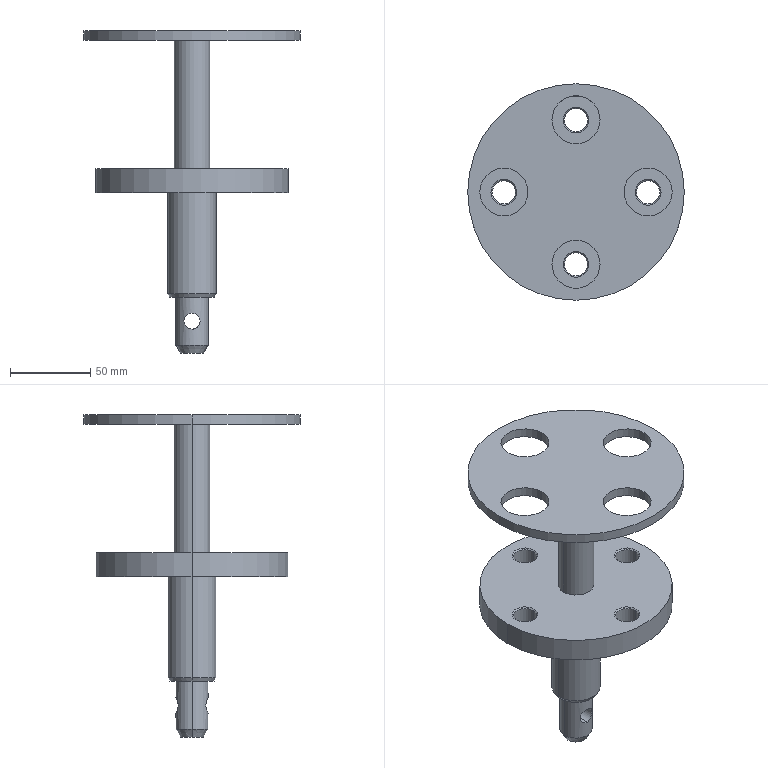Part | SolidWorks | features ICE 7, Chamfer 2, 3DProfileFeature 1, CirPattern 1, Extrusion 1, HoleWzd 1 | 1 solid | 46 faces | box 135 x 135 x 201 mm | volume 313916 mm3 | cylinder 28 | cone 12 | plane 6 | commonest cylinder face diameters 30 x10 14.5 x8 10 x2 20 x2 22 x2 120 x2
STEP:
#1=CARTESIAN_POINT('',(-60.,0.,215.));
#2=VERTEX_POINT('',#1);
#3=CARTESIAN_POINT('',(-30.,0.,215.));
#4=VERTEX_POINT('',#3);
#5=CARTESIAN_POINT('',(-45.,0.,215.));
#6=DIRECTION('',(0.,0.,1.));
#7=DIRECTION('',(1.,0.,0.));
#8=AXIS2_PLACEMENT_3D('',#5,#6,#7);
#9=CIRCLE('',#8,15.);
#10=EDGE_CURVE('',#2,#4,#9,.T.);
#11=ORIENTED_EDGE('',*,*,#10,.T.);
#12=CARTESIAN_POINT('',(-30.,0.,209.));
#13=VERTEX_POINT('',#12);
#14=CARTESIAN_POINT('',(-30.,0.,215.));
#15=DIRECTION('',(0.,0.,-1.));
#16=VECTOR('',#15,1000.);
#17=LINE('',#14,#16);
#18=EDGE_CURVE('',#4,#13,#17,.T.);
#19=ORIENTED_EDGE('',*,*,#18,.T.);
#20=CARTESIAN_POINT('',(-60.,0.,209.));
#21=VERTEX_POINT('',#20);
#22=CARTESIAN_POINT('',(-45.,0.,209.));
#23=DIRECTION('',(0.,0.,1.));
#24=DIRECTION('',(1.,0.,0.));
#25=AXIS2_PLACEMENT_3D('',#22,#23,#24);
#26=CIRCLE('',#25,15.);
#27=EDGE_CURVE('',#21,#13,#26,.T.);
#28=ORIENTED_EDGE('',*,*,#27,.F.);
#29=CARTESIAN_POINT('',(-60.,0.,215.));
#30=DIRECTION('',(0.,0.,-1.));
#31=VECTOR('',#30,1000.);
#32=LINE('',#29,#31);
#33=EDGE_CURVE('',#2,#21,#32,.T.);
#34=ORIENTED_EDGE('',*,*,#33,.F.);
#35=EDGE_LOOP('',(#11,#19,#28,#34));
#36=FACE_OUTER_BOUND('',#35,.T.);
#37=CARTESIAN_POINT('',(-45.,0.,215.));
#38=DIRECTION('',(0.,0.,-1.));
#39=DIRECTION('',(-1.,0.,0.));
#40=AXIS2_PLACEMENT_3D('',#37,#38,#39);
#41=CYLINDRICAL_SURFACE('',#40,15.);
#42=ADVANCED_FACE('',(#36),#41,.F.);
#43=CARTESIAN_POINT('',(-15.,-45.,215.));
#44=VERTEX_POINT('',#43);
#45=CARTESIAN_POINT('',(15.,-45.,215.));
#46=VERTEX_POINT('',#45);
#47=CARTESIAN_POINT('',(0.,-45.,215.));
#48=DIRECTION('',(0.,0.,1.));
#49=DIRECTION('',(1.,0.,0.));
#50=AXIS2_PLACEMENT_3D('',#47,#48,#49);
#51=CIRCLE('',#50,15.);
#52=EDGE_CURVE('',#44,#46,#51,.T.);
#53=ORIENTED_EDGE('',*,*,#52,.T.);
#54=CARTESIAN_POINT('',(15.,-45.,209.));
#55=VERTEX_POINT('',#54);
#56=CARTESIAN_POINT('',(15.,-45.,215.));
#57=DIRECTION('',(0.,0.,-1.));
#58=VECTOR('',#57,1000.);
#59=LINE('',#56,#58);
#60=EDGE_CURVE('',#46,#55,#59,.T.);
#61=ORIENTED_EDGE('',*,*,#60,.T.);
#62=CARTESIAN_POINT('',(-15.,-45.,209.));
#63=VERTEX_POINT('',#62);
#64=CARTESIAN_POINT('',(0.,-45.,209.));
#65=DIRECTION('',(0.,0.,1.));
#66=DIRECTION('',(1.,0.,0.));
#67=AXIS2_PLACEMENT_3D('',#64,#65,#66);
#68=CIRCLE('',#67,15.);
#69=EDGE_CURVE('',#63,#55,#68,.T.);
#70=ORIENTED_EDGE('',*,*,#69,.F.);
#71=CARTESIAN_POINT('',(-15.,-45.,215.));
#72=DIRECTION('',(0.,0.,-1.));
#73=VECTOR('',#72,1000.);
#74=LINE('',#71,#73);
#75=EDGE_CURVE('',#44,#63,#74,.T.);
#76=ORIENTED_EDGE('',*,*,#75,.F.);
#77=EDGE_LOOP('',(#53,#61,#70,#76));
#78=FACE_OUTER_BOUND('',#77,.T.);
#79=CARTESIAN_POINT('',(0.,-45.,215.));
#80=DIRECTION('',(0.,0.,-1.));
#81=DIRECTION('',(-1.,0.,0.));
#82=AXIS2_PLACEMENT_3D('',#79,#80,#81);
#83=CYLINDRICAL_SURFACE('',#82,15.);
#84=ADVANCED_FACE('',(#78),#83,.F.);
#85=CARTESIAN_POINT('',(30.,0.,215.));
#86=VERTEX_POINT('',#85);
#87=CARTESIAN_POINT('',(60.,0.,215.));
#88=VERTEX_POINT('',#87);
#89=CARTESIAN_POINT('',(45.,0.,215.));
#90=DIRECTION('',(0.,0.,1.));
#91=DIRECTION('',(1.,0.,0.));
#92=AXIS2_PLACEMENT_3D('',#89,#90,#91);
#93=CIRCLE('',#92,15.);
#94=EDGE_CURVE('',#86,#88,#93,.T.);
#95=ORIENTED_EDGE('',*,*,#94,.T.);
#96=CARTESIAN_POINT('',(60.,0.,209.));
#97=VERTEX_POINT('',#96);
#98=CARTESIAN_POINT('',(60.,0.,215.));
#99=DIRECTION('',(0.,0.,-1.));
#100=VECTOR('',#99,1000.);
#101=LINE('',#98,#100);
#102=EDGE_CURVE('',#88,#97,#101,.T.);
#103=ORIENTED_EDGE('',*,*,#102,.T.);
#104=CARTESIAN_POINT('',(30.,0.,209.));
#105=VERTEX_POINT('',#104);
#106=CARTESIAN_POINT('',(45.,0.,209.));
#107=DIRECTION('',(0.,0.,1.));
#108=DIRECTION('',(1.,0.,0.));
#109=AXIS2_PLACEMENT_3D('',#106,#107,#108);
#110=CIRCLE('',#109,15.);
#111=EDGE_CURVE('',#105,#97,#110,.T.);
#112=ORIENTED_EDGE('',*,*,#111,.F.);
#113=CARTESIAN_POINT('',(30.,0.,215.));
#114=DIRECTION('',(0.,0.,-1.));
#115=VECTOR('',#114,1000.);
#116=LINE('',#113,#115);
#117=EDGE_CURVE('',#86,#105,#116,.T.);
#118=ORIENTED_EDGE('',*,*,#117,.F.);
#119=EDGE_LOOP('',(#95,#103,#112,#118));
#120=FACE_OUTER_BOUND('',#119,.T.);
#121=CARTESIAN_POINT('',(45.,0.,215.));
#122=DIRECTION('',(0.,0.,-1.));
#123=DIRECTION('',(-1.,0.,0.));
#124=AXIS2_PLACEMENT_3D('',#121,#122,#123);
#125=CYLINDRICAL_SURFACE('',#124,15.);
#126=ADVANCED_FACE('',(#120),#125,.F.);
#127=CARTESIAN_POINT('',(-15.,45.,215.));
#128=VERTEX_POINT('',#127);
#129=CARTESIAN_POINT('',(15.,45.,215.));
#130=VERTEX_POINT('',#129);
#131=CARTESIAN_POINT('',(0.,45.,215.));
#132=DIRECTION('',(0.,0.,1.));
#133=DIRECTION('',(1.,0.,0.));
#134=AXIS2_PLACEMENT_3D('',#131,#132,#133);
#135=CIRCLE('',#134,15.);
#136=EDGE_CURVE('',#128,#130,#135,.T.);
#137=ORIENTED_EDGE('',*,*,#136,.T.);
#138=CARTESIAN_POINT('',(15.,45.,209.));
#139=VERTEX_POINT('',#138);
#140=CARTESIAN_POINT('',(15.,45.,215.));
#141=DIRECTION('',(0.,0.,-1.));
#142=VECTOR('',#141,1000.);
#143=LINE('',#140,#142);
#144=EDGE_CURVE('',#130,#139,#143,.T.);
#145=ORIENTED_EDGE('',*,*,#144,.T.);
#146=CARTESIAN_POINT('',(-15.,45.,209.));
#147=VERTEX_POINT('',#146);
#148=CARTESIAN_POINT('',(0.,45.,209.));
#149=DIRECTION('',(0.,0.,1.));
#150=DIRECTION('',(1.,0.,0.));
#151=AXIS2_PLACEMENT_3D('',#148,#149,#150);
#152=CIRCLE('',#151,15.);
#153=EDGE_CURVE('',#147,#139,#152,.T.);
#154=ORIENTED_EDGE('',*,*,#153,.F.);
#155=CARTESIAN_POINT('',(-15.,45.,215.));
#156=DIRECTION('',(0.,0.,-1.));
#157=VECTOR('',#156,1000.);
#158=LINE('',#155,#157);
#159=EDGE_CURVE('',#128,#147,#158,.T.);
#160=ORIENTED_EDGE('',*,*,#159,.F.);
#161=EDGE_LOOP('',(#137,#145,#154,#160));
#162=FACE_OUTER_BOUND('',#161,.T.);
#163=CARTESIAN_POINT('',(0.,45.,215.));
#164=DIRECTION('',(0.,0.,-1.));
#165=DIRECTION('',(-1.,0.,0.));
#166=AXIS2_PLACEMENT_3D('',#163,#164,#165);
#167=CYLINDRICAL_SURFACE('',#166,15.);
#168=ADVANCED_FACE('',(#162),#167,.F.);
#169=CARTESIAN_POINT('',(67.5,0.,215.));
#170=VERTEX_POINT('',#169);
#171=CARTESIAN_POINT('',(-67.5,0.,215.));
#172=VERTEX_POINT('',#171);
#173=CARTESIAN_POINT('',(0.,0.,215.));
#174=DIRECTION('',(0.,0.,1.));
#175=DIRECTION('',(1.,0.,0.));
#176=AXIS2_PLACEMENT_3D('',#173,#174,#175);
#177=CIRCLE('',#176,67.5);
#178=EDGE_CURVE('',#170,#172,#177,.T.);
#179=ORIENTED_EDGE('',*,*,#178,.F.);
#180=CARTESIAN_POINT('',(67.5,0.,209.));
#181=VERTEX_POINT('',#180);
#182=CARTESIAN_POINT('',(67.5,0.,215.));
#183=DIRECTION('',(0.,0.,-1.));
#184=VECTOR('',#183,1000.);
#185=LINE('',#182,#184);
#186=EDGE_CURVE('',#170,#181,#185,.T.);
#187=ORIENTED_EDGE('',*,*,#186,.T.);
#188=CARTESIAN_POINT('',(-67.5,0.,209.));
#189=VERTEX_POINT('',#188);
#190=CARTESIAN_POINT('',(0.,0.,209.));
#191=DIRECTION('',(0.,0.,1.));
#192=DIRECTION('',(1.,0.,0.));
#193=AXIS2_PLACEMENT_3D('',#190,#191,#192);
#194=CIRCLE('',#193,67.5);
#195=EDGE_CURVE('',#181,#189,#194,.T.);
#196=ORIENTED_EDGE('',*,*,#195,.T.);
#197=CARTESIAN_POINT('',(-67.5,0.,215.));
#198=DIRECTION('',(0.,0.,-1.));
#199=VECTOR('',#198,1000.);
#200=LINE('',#197,#199);
#201=EDGE_CURVE('',#172,#189,#200,.T.);
#202=ORIENTED_EDGE('',*,*,#201,.F.);
#203=EDGE_LOOP('',(#179,#187,#196,#202));
#204=FACE_OUTER_BOUND('',#203,.T.);
#205=CARTESIAN_POINT('',(0.,0.,215.));
#206=DIRECTION('',(0.,0.,-1.));
#207=DIRECTION('',(-1.,0.,0.));
#208=AXIS2_PLACEMENT_3D('',#205,#206,#207);
#209=CYLINDRICAL_SURFACE('',#208,67.5);
#210=ADVANCED_FACE('',(#204),#209,.T.);
#211=CARTESIAN_POINT('',(11.,0.,209.));
#212=VERTEX_POINT('',#211);
#213=CARTESIAN_POINT('',(-11.,0.,209.));
#214=VERTEX_POINT('',#213);
#215=CARTESIAN_POINT('',(0.,0.,209.));
#216=DIRECTION('',(0.,0.,1.));
#217=DIRECTION('',(1.,0.,0.));
#218=AXIS2_PLACEMENT_3D('',#215,#216,#217);
#219=CIRCLE('',#218,11.);
#220=EDGE_CURVE('',#212,#214,#219,.T.);
#221=ORIENTED_EDGE('',*,*,#220,.F.);
#222=CARTESIAN_POINT('',(11.,0.,129.));
#223=VERTEX_POINT('',#222);
#224=CARTESIAN_POINT('',(11.,0.,209.));
#225=DIRECTION('',(0.,0.,-1.));
#226=VECTOR('',#225,1000.);
#227=LINE('',#224,#226);
#228=EDGE_CURVE('',#212,#223,#227,.T.);
#229=ORIENTED_EDGE('',*,*,#228,.T.);
#230=CARTESIAN_POINT('',(-11.,0.,129.));
#231=VERTEX_POINT('',#230);
#232=CARTESIAN_POINT('',(0.,0.,129.));
#233=DIRECTION('',(0.,0.,1.));
#234=DIRECTION('',(1.,0.,0.));
#235=AXIS2_PLACEMENT_3D('',#232,#233,#234);
#236=CIRCLE('',#235,11.);
#237=EDGE_CURVE('',#223,#231,#236,.T.);
#238=ORIENTED_EDGE('',*,*,#237,.T.);
#239=CARTESIAN_POINT('',(-11.,0.,209.));
#240=DIRECTION('',(0.,0.,-1.));
#241=VECTOR('',#240,1000.);
#242=LINE('',#239,#241);
#243=EDGE_CURVE('',#214,#231,#242,.T.);
#244=ORIENTED_EDGE('',*,*,#243,.F.);
#245=EDGE_LOOP('',(#221,#229,#238,#244));
#246=FACE_OUTER_BOUND('',#245,.T.);
#247=CARTESIAN_POINT('',(0.,0.,209.));
#248=DIRECTION('',(0.,0.,-1.));
#249=DIRECTION('',(-1.,0.,0.));
#250=AXIS2_PLACEMENT_3D('',#247,#248,#249);
#251=CYLINDRICAL_SURFACE('',#250,11.);
#252=ADVANCED_FACE('',(#246),#251,.T.);
#253=CARTESIAN_POINT('',(-13.845,0.,49.));
#254=VERTEX_POINT('',#253);
#255=CARTESIAN_POINT('',(13.845,0.,49.));
#256=VERTEX_POINT('',#255);
#257=CARTESIAN_POINT('',(0.,0.,49.));
#258=DIRECTION('',(0.,0.,-1.));
#259=DIRECTION('',(-1.,0.,0.));
#260=AXIS2_PLACEMENT_3D('',#257,#258,#259);
#261=CIRCLE('',#260,13.845);
#262=EDGE_CURVE('',#254,#256,#261,.T.);
#263=ORIENTED_EDGE('',*,*,#262,.F.);
#264=CARTESIAN_POINT('',(-15.,0.,51.));
#265=VERTEX_POINT('',#264);
#266=CARTESIAN_POINT('',(-13.845,0.,49.));
#267=DIRECTION('',(-0.5,0.,0.866));
#268=VECTOR('',#267,1000.);
#269=LINE('',#266,#268);
#270=EDGE_CURVE('',#254,#265,#269,.T.);
#271=ORIENTED_EDGE('',*,*,#270,.T.);
#272=CARTESIAN_POINT('',(15.,0.,51.));
#273=VERTEX_POINT('',#272);
#274=CARTESIAN_POINT('',(0.,0.,51.));
#275=DIRECTION('',(0.,0.,1.));
#276=DIRECTION('',(-1.,0.,0.));
#277=AXIS2_PLACEMENT_3D('',#274,#275,#276);
#278=CIRCLE('',#277,15.);
#279=EDGE_CURVE('',#273,#265,#278,.T.);
#280=ORIENTED_EDGE('',*,*,#279,.F.);
#281=CARTESIAN_POINT('',(13.845,0.,49.));
#282=DIRECTION('',(0.5,0.,0.866));
#283=VECTOR('',#282,1000.);
#284=LINE('',#281,#283);
#285=EDGE_CURVE('',#256,#273,#284,.T.);
#286=ORIENTED_EDGE('',*,*,#285,.F.);
#287=EDGE_LOOP('',(#263,#271,#280,#286));
#288=FACE_OUTER_BOUND('',#287,.T.);
#289=CARTESIAN_POINT('',(0.,0.,49.));
#290=DIRECTION('',(0.,0.,1.));
#291=DIRECTION('',(1.,0.,0.));
#292=AXIS2_PLACEMENT_3D('',#289,#290,#291);
#293=CONICAL_SURFACE('',#292,13.845,0.5236);
#294=ADVANCED_FACE('',(#288),#293,.T.);
#295=CARTESIAN_POINT('',(37.75,0.,114.));
#296=VERTEX_POINT('',#295);
#297=CARTESIAN_POINT('',(52.25,0.,114.));
#298=VERTEX_POINT('',#297);
#299=CARTESIAN_POINT('',(45.,0.,114.));
#300=DIRECTION('',(0.,0.,1.));
#301=DIRECTION('',(1.,0.,0.));
#302=AXIS2_PLACEMENT_3D('',#299,#300,#301);
#303=CIRCLE('',#302,7.25);
#304=EDGE_CURVE('',#296,#298,#303,.T.);
#305=ORIENTED_EDGE('',*,*,#304,.F.);
#306=CARTESIAN_POINT('',(37.75,0.,128.225));
#307=VERTEX_POINT('',#306);
#308=CARTESIAN_POINT('',(37.75,0.,129.));
#309=DIRECTION('',(0.,0.,1.));
#310=VECTOR('',#309,1000.);
#311=LINE('',#308,#310);
#312=EDGE_CURVE('',#296,#307,#311,.T.);
#313=ORIENTED_EDGE('',*,*,#312,.T.);
#314=CARTESIAN_POINT('',(52.25,0.,128.225));
#315=VERTEX_POINT('',#314);
#316=CARTESIAN_POINT('',(45.,0.,128.225));
#317=DIRECTION('',(0.,0.,1.));
#318=DIRECTION('',(1.,0.,0.));
#319=AXIS2_PLACEMENT_3D('',#316,#317,#318);
#320=CIRCLE('',#319,7.25);
#321=EDGE_CURVE('',#307,#315,#320,.T.);
#322=ORIENTED_EDGE('',*,*,#321,.T.);
#323=CARTESIAN_POINT('',(52.25,0.,129.));
#324=DIRECTION('',(0.,0.,1.));
#325=VECTOR('',#324,1000.);
#326=LINE('',#323,#325);
#327=EDGE_CURVE('',#298,#315,#326,.T.);
#328=ORIENTED_EDGE('',*,*,#327,.F.);
#329=EDGE_LOOP('',(#305,#313,#322,#328));
#330=FACE_OUTER_BOUND('',#329,.T.);
#331=CARTESIAN_POINT('',(45.,0.,129.));
#332=DIRECTION('',(0.,0.,1.));
#333=DIRECTION('',(1.,0.,0.));
#334=AXIS2_PLACEMENT_3D('',#331,#332,#333);
#335=CYLINDRICAL_SURFACE('',#334,7.25);
#336=ADVANCED_FACE('',(#330),#335,.F.);
#337=CARTESIAN_POINT('',(-7.25,-45.,114.));
#338=VERTEX_POINT('',#337);
#339=CARTESIAN_POINT('',(7.25,-45.,114.));
#340=VERTEX_POINT('',#339);
#341=CARTESIAN_POINT('',(0.,-45.,114.));
#342=DIRECTION('',(0.,0.,1.));
#343=DIRECTION('',(1.,0.,0.));
#344=AXIS2_PLACEMENT_3D('',#341,#342,#343);
#345=CIRCLE('',#344,7.25);
#346=EDGE_CURVE('',#338,#340,#345,.T.);
#347=ORIENTED_EDGE('',*,*,#346,.F.);
#348=CARTESIAN_POINT('',(-7.25,-45.,128.225));
#349=VERTEX_POINT('',#348);
#350=CARTESIAN_POINT('',(-7.25,-45.,129.));
#351=DIRECTION('',(0.,0.,1.));
#352=VECTOR('',#351,1000.);
#353=LINE('',#350,#352);
#354=EDGE_CURVE('',#338,#349,#353,.T.);
#355=ORIENTED_EDGE('',*,*,#354,.T.);
#356=CARTESIAN_POINT('',(7.25,-45.,128.225));
#357=VERTEX_POINT('',#356);
#358=CARTESIAN_POINT('',(0.,-45.,128.225));
#359=DIRECTION('',(0.,0.,1.));
#360=DIRECTION('',(1.,0.,0.));
#361=AXIS2_PLACEMENT_3D('',#358,#359,#360);
#362=CIRCLE('',#361,7.25);
#363=EDGE_CURVE('',#349,#357,#362,.T.);
#364=ORIENTED_EDGE('',*,*,#363,.T.);
#365=CARTESIAN_POINT('',(7.25,-45.,129.));
#366=DIRECTION('',(0.,0.,1.));
#367=VECTOR('',#366,1000.);
#368=LINE('',#365,#367);
#369=EDGE_CURVE('',#340,#357,#368,.T.);
#370=ORIENTED_EDGE('',*,*,#369,.F.);
#371=EDGE_LOOP('',(#347,#355,#364,#370));
#372=FACE_OUTER_BOUND('',#371,.T.);
#373=CARTESIAN_POINT('',(0.,-45.,129.));
#374=DIRECTION('',(0.,0.,1.));
#375=DIRECTION('',(1.,0.,0.));
#376=AXIS2_PLACEMENT_3D('',#373,#374,#375);
#377=CYLINDRICAL_SURFACE('',#376,7.25);
#378=ADVANCED_FACE('',(#372),#377,.F.);
#379=CARTESIAN_POINT('',(-52.25,0.,114.));
#380=VERTEX_POINT('',#379);
#381=CARTESIAN_POINT('',(-37.75,0.,114.));
#382=VERTEX_POINT('',#381);
#383=CARTESIAN_POINT('',(-45.,0.,114.));
#384=DIRECTION('',(0.,0.,1.));
#385=DIRECTION('',(1.,0.,0.));
#386=AXIS2_PLACEMENT_3D('',#383,#384,#385);
#387=CIRCLE('',#386,7.25);
#388=EDGE_CURVE('',#380,#382,#387,.T.);
#389=ORIENTED_EDGE('',*,*,#388,.F.);
#390=CARTESIAN_POINT('',(-52.25,0.,128.225));
#391=VERTEX_POINT('',#390);
#392=CARTESIAN_POINT('',(-52.25,0.,129.));
#393=DIRECTION('',(0.,0.,1.));
#394=VECTOR('',#393,1000.);
#395=LINE('',#392,#394);
#396=EDGE_CURVE('',#380,#391,#395,.T.);
#397=ORIENTED_EDGE('',*,*,#396,.T.);
#398=CARTESIAN_POINT('',(-37.75,0.,128.225));
#399=VERTEX_POINT('',#398);
#400=CARTESIAN_POINT('',(-45.,0.,128.225));
#401=DIRECTION('',(0.,0.,1.));
#402=DIRECTION('',(1.,0.,0.));
#403=AXIS2_PLACEMENT_3D('',#400,#401,#402);
#404=CIRCLE('',#403,7.25);
#405=EDGE_CURVE('',#391,#399,#404,.T.);
#406=ORIENTED_EDGE('',*,*,#405,.T.);
#407=CARTESIAN_POINT('',(-37.75,0.,129.));
#408=DIRECTION('',(0.,0.,1.));
#409=VECTOR('',#408,1000.);
#410=LINE('',#407,#409);
#411=EDGE_CURVE('',#382,#399,#410,.T.);
#412=ORIENTED_EDGE('',*,*,#411,.F.);
#413=EDGE_LOOP('',(#389,#397,#406,#412));
#414=FACE_OUTER_BOUND('',#413,.T.);
#415=CARTESIAN_POINT('',(-45.,0.,129.));
#416=DIRECTION('',(0.,0.,1.));
#417=DIRECTION('',(1.,0.,0.));
#418=AXIS2_PLACEMENT_3D('',#415,#416,#417);
#419=CYLINDRICAL_SURFACE('',#418,7.25);
#420=ADVANCED_FACE('',(#414),#419,.F.);
#421=CARTESIAN_POINT('',(-7.25,45.,114.));
#422=VERTEX_POINT('',#421);
#423=CARTESIAN_POINT('',(7.25,45.,114.));
#424=VERTEX_POINT('',#423);
#425=CARTESIAN_POINT('',(0.,45.,114.));
#426=DIRECTION('',(0.,0.,1.));
#427=DIRECTION('',(1.,0.,0.));
#428=AXIS2_PLACEMENT_3D('',#425,#426,#427);
#429=CIRCLE('',#428,7.25);
#430=EDGE_CURVE('',#422,#424,#429,.T.);
#431=ORIENTED_EDGE('',*,*,#430,.F.);
#432=CARTESIAN_POINT('',(-7.25,45.,128.225));
#433=VERTEX_POINT('',#432);
#434=CARTESIAN_POINT('',(-7.25,45.,129.));
#435=DIRECTION('',(0.,0.,1.));
#436=VECTOR('',#435,1000.);
#437=LINE('',#434,#436);
#438=EDGE_CURVE('',#422,#433,#437,.T.);
#439=ORIENTED_EDGE('',*,*,#438,.T.);
#440=CARTESIAN_POINT('',(7.25,45.,128.225));
#441=VERTEX_POINT('',#440);
#442=CARTESIAN_POINT('',(0.,45.,128.225));
#443=DIRECTION('',(0.,0.,1.));
#444=DIRECTION('',(1.,0.,0.));
#445=AXIS2_PLACEMENT_3D('',#442,#443,#444);
#446=CIRCLE('',#445,7.25);
#447=EDGE_CURVE('',#433,#441,#446,.T.);
#448=ORIENTED_EDGE('',*,*,#447,.T.);
#449=CARTESIAN_POINT('',(7.25,45.,129.));
#450=DIRECTION('',(0.,0.,1.));
#451=VECTOR('',#450,1000.);
#452=LINE('',#449,#451);
#453=EDGE_CURVE('',#424,#441,#452,.T.);
#454=ORIENTED_EDGE('',*,*,#453,.F.);
#455=EDGE_LOOP('',(#431,#439,#448,#454));
#456=FACE_OUTER_BOUND('',#455,.T.);
#457=CARTESIAN_POINT('',(0.,45.,129.));
#458=DIRECTION('',(0.,0.,1.));
#459=DIRECTION('',(1.,0.,0.));
#460=AXIS2_PLACEMENT_3D('',#457,#458,#459);
#461=CYLINDRICAL_SURFACE('',#460,7.25);
#462=ADVANCED_FACE('',(#456),#461,.F.);
#463=CARTESIAN_POINT('',(60.,0.,129.));
#464=VERTEX_POINT('',#463);
#465=CARTESIAN_POINT('',(-60.,0.,129.));
#466=VERTEX_POINT('',#465);
#467=CARTESIAN_POINT('',(0.,0.,129.));
#468=DIRECTION('',(0.,0.,1.));
#469=DIRECTION('',(1.,0.,0.));
#470=AXIS2_PLACEMENT_3D('',#467,#468,#469);
#471=CIRCLE('',#470,60.);
#472=EDGE_CURVE('',#464,#466,#471,.T.);
#473=ORIENTED_EDGE('',*,*,#472,.F.);
#474=CARTESIAN_POINT('',(60.,0.,114.));
#475=VERTEX_POINT('',#474);
#476=CARTESIAN_POINT('',(60.,0.,129.));
#477=DIRECTION('',(0.,0.,-1.));
#478=VECTOR('',#477,1000.);
#479=LINE('',#476,#478);
#480=EDGE_CURVE('',#464,#475,#479,.T.);
#481=ORIENTED_EDGE('',*,*,#480,.T.);
#482=CARTESIAN_POINT('',(-60.,0.,114.));
#483=VERTEX_POINT('',#482);
#484=CARTESIAN_POINT('',(0.,0.,114.));
#485=DIRECTION('',(0.,0.,1.));
#486=DIRECTION('',(1.,0.,0.));
#487=AXIS2_PLACEMENT_3D('',#484,#485,#486);
#488=CIRCLE('',#487,60.);
#489=EDGE_CURVE('',#475,#483,#488,.T.);
#490=ORIENTED_EDGE('',*,*,#489,.T.);
#491=CARTESIAN_POINT('',(-60.,0.,129.));
#492=DIRECTION('',(0.,0.,-1.));
#493=VECTOR('',#492,1000.);
#494=LINE('',#491,#493);
#495=EDGE_CURVE('',#466,#483,#494,.T.);
#496=ORIENTED_EDGE('',*,*,#495,.F.);
#497=EDGE_LOOP('',(#473,#481,#490,#496));
#498=FACE_OUTER_BOUND('',#497,.T.);
#499=CARTESIAN_POINT('',(0.,0.,129.));
#500=DIRECTION('',(0.,0.,-1.));
#501=DIRECTION('',(-1.,0.,0.));
#502=AXIS2_PLACEMENT_3D('',#499,#500,#501);
#503=CYLINDRICAL_SURFACE('',#502,60.);
#504=ADVANCED_FACE('',(#498),#503,.T.);
#505=ORIENTED_EDGE('',*,*,#321,.F.);
#506=CARTESIAN_POINT('',(36.975,0.,129.));
#507=VERTEX_POINT('',#506);
#508=CARTESIAN_POINT('',(36.975,0.,129.));
#509=DIRECTION('',(-0.7071,0.,0.7071));
#510=VECTOR('',#509,1000.);
#511=LINE('',#508,#510);
#512=EDGE_CURVE('',#307,#507,#511,.T.);
#513=ORIENTED_EDGE('',*,*,#512,.T.);
#514=CARTESIAN_POINT('',(53.025,0.,129.));
#515=VERTEX_POINT('',#514);
#516=CARTESIAN_POINT('',(45.,0.,129.));
#517=DIRECTION('',(0.,0.,1.));
#518=DIRECTION('',(1.,0.,0.));
#519=AXIS2_PLACEMENT_3D('',#516,#517,#518);
#520=CIRCLE('',#519,8.025);
#521=EDGE_CURVE('',#507,#515,#520,.T.);
#522=ORIENTED_EDGE('',*,*,#521,.T.);
#523=CARTESIAN_POINT('',(53.025,0.,129.));
#524=DIRECTION('',(0.7071,0.,0.7071));
#525=VECTOR('',#524,1000.);
#526=LINE('',#523,#525);
#527=EDGE_CURVE('',#315,#515,#526,.T.);
#528=ORIENTED_EDGE('',*,*,#527,.F.);
#529=EDGE_LOOP('',(#505,#513,#522,#528));
#530=FACE_OUTER_BOUND('',#529,.T.);
#531=CARTESIAN_POINT('',(45.,0.,129.));
#532=DIRECTION('',(0.,0.,1.));
#533=DIRECTION('',(1.,0.,0.));
#534=AXIS2_PLACEMENT_3D('',#531,#532,#533);
#535=CONICAL_SURFACE('',#534,8.025,0.7854);
#536=ADVANCED_FACE('',(#530),#535,.F.);
#537=ORIENTED_EDGE('',*,*,#363,.F.);
#538=CARTESIAN_POINT('',(-8.025,-45.,129.));
#539=VERTEX_POINT('',#538);
#540=CARTESIAN_POINT('',(-8.025,-45.,129.));
#541=DIRECTION('',(-0.7071,0.,0.7071));
#542=VECTOR('',#541,1000.);
#543=LINE('',#540,#542);
#544=EDGE_CURVE('',#349,#539,#543,.T.);
#545=ORIENTED_EDGE('',*,*,#544,.T.);
#546=CARTESIAN_POINT('',(8.025,-45.,129.));
#547=VERTEX_POINT('',#546);
#548=CARTESIAN_POINT('',(0.,-45.,129.));
#549=DIRECTION('',(0.,0.,1.));
#550=DIRECTION('',(1.,0.,0.));
#551=AXIS2_PLACEMENT_3D('',#548,#549,#550);
#552=CIRCLE('',#551,8.025);
#553=EDGE_CURVE('',#539,#547,#552,.T.);
#554=ORIENTED_EDGE('',*,*,#553,.T.);
#555=CARTESIAN_POINT('',(8.025,-45.,129.));
#556=DIRECTION('',(0.7071,0.,0.7071));
#557=VECTOR('',#556,1000.);
#558=LINE('',#555,#557);
#559=EDGE_CURVE('',#357,#547,#558,.T.);
#560=ORIENTED_EDGE('',*,*,#559,.F.);
#561=EDGE_LOOP('',(#537,#545,#554,#560));
#562=FACE_OUTER_BOUND('',#561,.T.);
#563=CARTESIAN_POINT('',(0.,-45.,129.));
#564=DIRECTION('',(0.,0.,1.));
#565=DIRECTION('',(1.,0.,0.));
#566=AXIS2_PLACEMENT_3D('',#563,#564,#565);
#567=CONICAL_SURFACE('',#566,8.025,0.7854);
#568=ADVANCED_FACE('',(#562),#567,.F.);
#569=ORIENTED_EDGE('',*,*,#405,.F.);
#570=CARTESIAN_POINT('',(-53.025,0.,129.));
#571=VERTEX_POINT('',#570);
#572=CARTESIAN_POINT('',(-53.025,0.,129.));
#573=DIRECTION('',(-0.7071,0.,0.7071));
#574=VECTOR('',#573,1000.);
#575=LINE('',#572,#574);
#576=EDGE_CURVE('',#391,#571,#575,.T.);
#577=ORIENTED_EDGE('',*,*,#576,.T.);
#578=CARTESIAN_POINT('',(-36.975,0.,129.));
#579=VERTEX_POINT('',#578);
#580=CARTESIAN_POINT('',(-45.,0.,129.));
#581=DIRECTION('',(0.,0.,1.));
#582=DIRECTION('',(1.,0.,0.));
#583=AXIS2_PLACEMENT_3D('',#580,#581,#582);
#584=CIRCLE('',#583,8.025);
#585=EDGE_CURVE('',#571,#579,#584,.T.);
#586=ORIENTED_EDGE('',*,*,#585,.T.);
#587=CARTESIAN_POINT('',(-36.975,0.,129.));
#588=DIRECTION('',(0.7071,0.,0.7071));
#589=VECTOR('',#588,1000.);
#590=LINE('',#587,#589);
#591=EDGE_CURVE('',#399,#579,#590,.T.);
#592=ORIENTED_EDGE('',*,*,#591,.F.);
#593=EDGE_LOOP('',(#569,#577,#586,#592));
#594=FACE_OUTER_BOUND('',#593,.T.);
#595=CARTESIAN_POINT('',(-45.,0.,129.));
#596=DIRECTION('',(0.,0.,1.));
#597=DIRECTION('',(1.,0.,0.));
#598=AXIS2_PLACEMENT_3D('',#595,#596,#597);
#599=CONICAL_SURFACE('',#598,8.025,0.7854);
#600=ADVANCED_FACE('',(#594),#599,.F.);
#601=ORIENTED_EDGE('',*,*,#447,.F.);
#602=CARTESIAN_POINT('',(-8.025,45.,129.));
#603=VERTEX_POINT('',#602);
#604=CARTESIAN_POINT('',(-8.025,45.,129.));
#605=DIRECTION('',(-0.7071,0.,0.7071));
#606=VECTOR('',#605,1000.);
#607=LINE('',#604,#606);
#608=EDGE_CURVE('',#433,#603,#607,.T.);
#609=ORIENTED_EDGE('',*,*,#608,.T.);
#610=CARTESIAN_POINT('',(8.025,45.,129.));
#611=VERTEX_POINT('',#610);
#612=CARTESIAN_POINT('',(0.,45.,129.));
#613=DIRECTION('',(0.,0.,1.));
#614=DIRECTION('',(1.,0.,0.));
#615=AXIS2_PLACEMENT_3D('',#612,#613,#614);
#616=CIRCLE('',#615,8.025);
#617=EDGE_CURVE('',#603,#611,#616,.T.);
#618=ORIENTED_EDGE('',*,*,#617,.T.);
#619=CARTESIAN_POINT('',(8.025,45.,129.));
#620=DIRECTION('',(0.7071,0.,0.7071));
#621=VECTOR('',#620,1000.);
#622=LINE('',#619,#621);
#623=EDGE_CURVE('',#441,#611,#622,.T.);
#624=ORIENTED_EDGE('',*,*,#623,.F.);
#625=EDGE_LOOP('',(#601,#609,#618,#624));
#626=FACE_OUTER_BOUND('',#625,.T.);
#627=CARTESIAN_POINT('',(0.,45.,129.));
#628=DIRECTION('',(0.,0.,1.));
#629=DIRECTION('',(1.,0.,0.));
#630=AXIS2_PLACEMENT_3D('',#627,#628,#629);
#631=CONICAL_SURFACE('',#630,8.025,0.7854);
#632=ADVANCED_FACE('',(#626),#631,.F.);
#633=ORIENTED_EDGE('',*,*,#279,.T.);
#634=CARTESIAN_POINT('',(-15.,0.,114.));
#635=VERTEX_POINT('',#634);
#636=CARTESIAN_POINT('',(-15.,0.,49.));
#637=DIRECTION('',(0.,0.,1.));
#638=VECTOR('',#637,1000.);
#639=LINE('',#636,#638);
#640=EDGE_CURVE('',#265,#635,#639,.T.);
#641=ORIENTED_EDGE('',*,*,#640,.T.);
#642=CARTESIAN_POINT('',(15.,0.,114.));
#643=VERTEX_POINT('',#642);
#644=CARTESIAN_POINT('',(0.,0.,114.));
#645=DIRECTION('',(0.,0.,-1.));
#646=DIRECTION('',(1.,0.,0.));
#647=AXIS2_PLACEMENT_3D('',#644,#645,#646);
#648=CIRCLE('',#647,15.);
#649=EDGE_CURVE('',#635,#643,#648,.T.);
#650=ORIENTED_EDGE('',*,*,#649,.T.);
#651=CARTESIAN_POINT('',(15.,0.,49.));
#652=DIRECTION('',(0.,0.,1.));
#653=VECTOR('',#652,1000.);
#654=LINE('',#651,#653);
#655=EDGE_CURVE('',#273,#643,#654,.T.);
#656=ORIENTED_EDGE('',*,*,#655,.F.);
#657=EDGE_LOOP('',(#633,#641,#650,#656));
#658=FACE_OUTER_BOUND('',#657,.T.);
#659=CARTESIAN_POINT('',(0.,0.,49.));
#660=DIRECTION('',(0.,0.,1.));
#661=DIRECTION('',(1.,0.,0.));
#662=AXIS2_PLACEMENT_3D('',#659,#660,#661);
#663=CYLINDRICAL_SURFACE('',#662,15.);
#664=ADVANCED_FACE('',(#658),#663,.T.);
#665=CARTESIAN_POINT('',(0.,-10.,29.));
#666=VERTEX_POINT('',#665);
#667=CARTESIAN_POINT('',(0.,-10.,39.));
#668=VERTEX_POINT('',#667);
#669=CARTESIAN_POINT('',(0.,-10.,29.));
#670=CARTESIAN_POINT('',(-0.3314,-10.,29.));
#671=CARTESIAN_POINT('',(-0.6687,-9.983,29.034));
#672=CARTESIAN_POINT('',(-1.317,-9.918,29.165));
#673=CARTESIAN_POINT('',(-1.631,-9.871,29.262));
#674=CARTESIAN_POINT('',(-2.24,-9.751,29.518));
#675=CARTESIAN_POINT('',(-2.526,-9.68,29.673));
#676=CARTESIAN_POINT('',(-3.061,-9.524,30.034));
#677=CARTESIAN_POINT('',(-3.314,-9.438,30.242));
#678=CARTESIAN_POINT('',(-3.767,-9.266,30.697));
#679=CARTESIAN_POINT('',(-3.971,-9.18,30.944));
#680=CARTESIAN_POINT('',(-4.331,-9.016,31.48));
#681=CARTESIAN_POINT('',(-4.487,-8.938,31.769));
#682=CARTESIAN_POINT('',(-4.737,-8.808,32.367));
#683=CARTESIAN_POINT('',(-4.834,-8.754,32.679));
#684=CARTESIAN_POINT('',(-4.933,-8.699,33.168));
#685=CARTESIAN_POINT('',(-4.958,-8.684,33.334));
#686=CARTESIAN_POINT('',(-4.991,-8.665,33.664));
#687=CARTESIAN_POINT('',(-5.008,-8.656,33.994));
#688=CARTESIAN_POINT('',(-4.992,-8.665,34.325));
#689=CARTESIAN_POINT('',(-4.959,-8.684,34.657));
#690=CARTESIAN_POINT('',(-4.935,-8.698,34.823));
#691=CARTESIAN_POINT('',(-4.836,-8.753,35.311));
#692=CARTESIAN_POINT('',(-4.74,-8.806,35.625));
#693=CARTESIAN_POINT('',(-4.487,-8.938,36.23));
#694=CARTESIAN_POINT('',(-4.332,-9.015,36.518));
#695=CARTESIAN_POINT('',(-3.973,-9.179,37.053));
#696=CARTESIAN_POINT('',(-3.767,-9.267,37.304));
#697=CARTESIAN_POINT('',(-3.311,-9.439,37.761));
#698=CARTESIAN_POINT('',(-3.064,-9.523,37.965));
#699=CARTESIAN_POINT('',(-2.528,-9.679,38.326));
#700=CARTESIAN_POINT('',(-2.237,-9.751,38.483));
#701=CARTESIAN_POINT('',(-1.635,-9.87,38.736));
#702=CARTESIAN_POINT('',(-1.323,-9.918,38.833));
#703=CARTESIAN_POINT('',(-0.6735,-9.983,38.965));
#704=CARTESIAN_POINT('',(-0.3359,-10.,39.));
#705=CARTESIAN_POINT('',(0.,-10.,39.));
#706=B_SPLINE_CURVE_WITH_KNOTS('',3,(#669,#670,#671,#672,#673,#674,#675,#676,#677,#678,#679,#680,#681,#682,#683,#684,#685,#686,#687,#688,#689,#690,#691,#692,#693,#694,#695,#696,#697,#698,#699,#700,#701,#702,#703,#704,#705),.UNSPECIFIED.,.F.,.F.,(4,2,2,2,2,2,2,2,2,1,2,2,2,2,2,2,2,2,4),(0.0159,0.0169,0.01789,0.01888,0.01987,0.02087,0.02186,0.02285,0.02335,0.02384,0.02434,0.02484,0.02583,0.02682,0.02781,0.02881,0.0298,0.03079,0.03178),.UNSPECIFIED.);
#707=EDGE_CURVE('',#666,#668,#706,.T.);
#708=ORIENTED_EDGE('',*,*,#707,.F.);
#709=CARTESIAN_POINT('',(0.,10.,29.));
#710=VERTEX_POINT('',#709);
#711=CARTESIAN_POINT('',(0.,-60.,29.));
#712=DIRECTION('',(0.,1.,0.));
#713=VECTOR('',#712,1000.);
#714=LINE('',#711,#713);
#715=EDGE_CURVE('',#666,#710,#714,.T.);
#716=ORIENTED_EDGE('',*,*,#715,.T.);
#717=CARTESIAN_POINT('',(0.,10.,39.));
#718=VERTEX_POINT('',#717);
#719=CARTESIAN_POINT('',(0.,10.,39.));
#720=CARTESIAN_POINT('',(-0.3365,10.,39.));
#721=CARTESIAN_POINT('',(-0.6663,9.983,38.966));
#722=CARTESIAN_POINT('',(-1.314,9.919,38.836));
#723=CARTESIAN_POINT('',(-1.634,9.87,38.737));
#724=CARTESIAN_POINT('',(-2.238,9.751,38.483));
#725=CARTESIAN_POINT('',(-2.523,9.68,38.329));
#726=CARTESIAN_POINT('',(-3.063,9.524,37.965));
#727=CARTESIAN_POINT('',(-3.313,9.438,37.758));
#728=CARTESIAN_POINT('',(-3.766,9.267,37.305));
#729=CARTESIAN_POINT('',(-3.972,9.179,37.054));
#730=CARTESIAN_POINT('',(-4.333,9.015,36.516));
#731=CARTESIAN_POINT('',(-4.486,8.939,36.232));
#732=CARTESIAN_POINT('',(-4.674,8.841,35.783));
#733=CARTESIAN_POINT('',(-4.73,8.811,35.629));
#734=CARTESIAN_POINT('',(-4.827,8.758,35.313));
#735=CARTESIAN_POINT('',(-4.868,8.735,35.152));
#736=CARTESIAN_POINT('',(-4.966,8.68,34.666));
#737=CARTESIAN_POINT('',(-5.,8.66,34.338));
#738=CARTESIAN_POINT('',(-5.,8.66,33.838));
#739=CARTESIAN_POINT('',(-4.992,8.665,33.67));
#740=CARTESIAN_POINT('',(-4.959,8.684,33.337));
#741=CARTESIAN_POINT('',(-4.934,8.698,33.173));
#742=CARTESIAN_POINT('',(-4.836,8.753,32.688));
#743=CARTESIAN_POINT('',(-4.738,8.807,32.37));
#744=CARTESIAN_POINT('',(-4.485,8.939,31.765));
#745=CARTESIAN_POINT('',(-4.331,9.016,31.48));
#746=CARTESIAN_POINT('',(-3.97,9.18,30.943));
#747=CARTESIAN_POINT('',(-3.763,9.268,30.692));
#748=CARTESIAN_POINT('',(-3.309,9.44,30.238));
#749=CARTESIAN_POINT('',(-3.061,9.524,30.033));
#750=CARTESIAN_POINT('',(-2.52,9.681,29.669));
#751=CARTESIAN_POINT('',(-2.233,9.752,29.514));
#752=CARTESIAN_POINT('',(-1.783,9.841,29.326));
#753=CARTESIAN_POINT('',(-1.629,9.868,29.27));
#754=CARTESIAN_POINT('',(-1.314,9.915,29.173));
#755=CARTESIAN_POINT('',(-1.152,9.935,29.132));
#756=CARTESIAN_POINT('',(-0.6614,9.984,29.033));
#757=CARTESIAN_POINT('',(-0.332,10.,29.));
#758=CARTESIAN_POINT('',(0.,10.,29.));
#759=B_SPLINE_CURVE_WITH_KNOTS('',3,(#719,#720,#721,#722,#723,#724,#725,#726,#727,#728,#729,#730,#731,#732,#733,#734,#735,#736,#737,#738,#739,#740,#741,#742,#743,#744,#745,#746,#747,#748,#749,#750,#751,#752,#753,#754,#755,#756,#757,#758),.UNSPECIFIED.,.F.,.F.,(4,2,2,2,2,2,2,2,2,2,2,2,2,2,2,2,2,2,2,4),(0.,0.0009941,0.001988,0.002982,0.003976,0.00497,0.005964,0.006461,0.006958,0.007952,0.008449,0.008947,0.009941,0.01093,0.01193,0.01292,0.01392,0.01441,0.01491,0.0159),.UNSPECIFIED.);
#760=EDGE_CURVE('',#718,#710,#759,.T.);
#761=ORIENTED_EDGE('',*,*,#760,.F.);
#762=CARTESIAN_POINT('',(0.,-60.,39.));
#763=DIRECTION('',(0.,1.,0.));
#764=VECTOR('',#763,1000.);
#765=LINE('',#762,#764);
#766=EDGE_CURVE('',#668,#718,#765,.T.);
#767=ORIENTED_EDGE('',*,*,#766,.F.);
#768=EDGE_LOOP('',(#708,#716,#761,#767));
#769=FACE_OUTER_BOUND('',#768,.T.);
#770=CARTESIAN_POINT('',(0.,-60.,34.));
#771=DIRECTION('',(0.,1.,0.));
#772=DIRECTION('',(0.,0.,1.));
#773=AXIS2_PLACEMENT_3D('',#770,#771,#772);
#774=CYLINDRICAL_SURFACE('',#773,5.);
#775=ADVANCED_FACE('',(#769),#774,.F.);
#776=CARTESIAN_POINT('',(-7.113,0.,14.));
#777=VERTEX_POINT('',#776);
#778=CARTESIAN_POINT('',(7.113,0.,14.));
#779=VERTEX_POINT('',#778);
#780=CARTESIAN_POINT('',(0.,0.,14.));
#781=DIRECTION('',(0.,0.,-1.));
#782=DIRECTION('',(-1.,0.,0.));
#783=AXIS2_PLACEMENT_3D('',#780,#781,#782);
#784=CIRCLE('',#783,7.113);
#785=EDGE_CURVE('',#777,#779,#784,.T.);
#786=ORIENTED_EDGE('',*,*,#785,.F.);
#787=CARTESIAN_POINT('',(-10.,0.,19.));
#788=VERTEX_POINT('',#787);
#789=CARTESIAN_POINT('',(-7.113,0.,14.));
#790=DIRECTION('',(-0.5,0.,0.866));
#791=VECTOR('',#790,1000.);
#792=LINE('',#789,#791);
#793=EDGE_CURVE('',#777,#788,#792,.T.);
#794=ORIENTED_EDGE('',*,*,#793,.T.);
#795=CARTESIAN_POINT('',(10.,0.,19.));
#796=VERTEX_POINT('',#795);
#797=CARTESIAN_POINT('',(0.,0.,19.));
#798=DIRECTION('',(0.,0.,1.));
#799=DIRECTION('',(-1.,0.,0.));
#800=AXIS2_PLACEMENT_3D('',#797,#798,#799);
#801=CIRCLE('',#800,10.);
#802=EDGE_CURVE('',#796,#788,#801,.T.);
#803=ORIENTED_EDGE('',*,*,#802,.F.);
#804=CARTESIAN_POINT('',(7.113,0.,14.));
#805=DIRECTION('',(0.5,0.,0.866));
#806=VECTOR('',#805,1000.);
#807=LINE('',#804,#806);
#808=EDGE_CURVE('',#779,#796,#807,.T.);
#809=ORIENTED_EDGE('',*,*,#808,.F.);
#810=EDGE_LOOP('',(#786,#794,#803,#809));
#811=FACE_OUTER_BOUND('',#810,.T.);
#812=CARTESIAN_POINT('',(0.,0.,14.));
#813=DIRECTION('',(0.,0.,1.));
#814=DIRECTION('',(1.,0.,0.));
#815=AXIS2_PLACEMENT_3D('',#812,#813,#814);
#816=CONICAL_SURFACE('',#815,7.113,0.5236);
#817=ADVANCED_FACE('',(#811),#816,.T.);
#818=ORIENTED_EDGE('',*,*,#760,.T.);
#819=CARTESIAN_POINT('',(0.,10.,29.));
#820=CARTESIAN_POINT('',(0.3314,10.,29.));
#821=CARTESIAN_POINT('',(0.6687,9.983,29.034));
#822=CARTESIAN_POINT('',(1.317,9.918,29.165));
#823=CARTESIAN_POINT('',(1.631,9.871,29.262));
#824=CARTESIAN_POINT('',(2.24,9.751,29.518));
#825=CARTESIAN_POINT('',(2.526,9.68,29.673));
#826=CARTESIAN_POINT('',(3.061,9.524,30.034));
#827=CARTESIAN_POINT('',(3.314,9.438,30.242));
#828=CARTESIAN_POINT('',(3.767,9.266,30.697));
#829=CARTESIAN_POINT('',(3.971,9.18,30.944));
#830=CARTESIAN_POINT('',(4.331,9.016,31.48));
#831=CARTESIAN_POINT('',(4.487,8.938,31.769));
#832=CARTESIAN_POINT('',(4.737,8.808,32.367));
#833=CARTESIAN_POINT('',(4.834,8.754,32.679));
#834=CARTESIAN_POINT('',(4.933,8.699,33.168));
#835=CARTESIAN_POINT('',(4.958,8.684,33.334));
#836=CARTESIAN_POINT('',(4.991,8.665,33.664));
#837=CARTESIAN_POINT('',(5.008,8.656,33.994));
#838=CARTESIAN_POINT('',(4.992,8.665,34.325));
#839=CARTESIAN_POINT('',(4.959,8.684,34.657));
#840=CARTESIAN_POINT('',(4.935,8.698,34.823));
#841=CARTESIAN_POINT('',(4.836,8.753,35.311));
#842=CARTESIAN_POINT('',(4.74,8.806,35.625));
#843=CARTESIAN_POINT('',(4.487,8.938,36.23));
#844=CARTESIAN_POINT('',(4.332,9.015,36.518));
#845=CARTESIAN_POINT('',(3.973,9.179,37.053));
#846=CARTESIAN_POINT('',(3.767,9.267,37.304));
#847=CARTESIAN_POINT('',(3.311,9.439,37.761));
#848=CARTESIAN_POINT('',(3.064,9.523,37.965));
#849=CARTESIAN_POINT('',(2.528,9.679,38.326));
#850=CARTESIAN_POINT('',(2.237,9.751,38.483));
#851=CARTESIAN_POINT('',(1.635,9.87,38.736));
#852=CARTESIAN_POINT('',(1.323,9.918,38.833));
#853=CARTESIAN_POINT('',(0.6735,9.983,38.965));
#854=CARTESIAN_POINT('',(0.3359,10.,39.));
#855=CARTESIAN_POINT('',(0.,10.,39.));
#856=B_SPLINE_CURVE_WITH_KNOTS('',3,(#819,#820,#821,#822,#823,#824,#825,#826,#827,#828,#829,#830,#831,#832,#833,#834,#835,#836,#837,#838,#839,#840,#841,#842,#843,#844,#845,#846,#847,#848,#849,#850,#851,#852,#853,#854,#855),.UNSPECIFIED.,.F.,.F.,(4,2,2,2,2,2,2,2,2,1,2,2,2,2,2,2,2,2,4),(0.0159,0.0169,0.01789,0.01888,0.01987,0.02087,0.02186,0.02285,0.02335,0.02384,0.02434,0.02484,0.02583,0.02682,0.02781,0.02881,0.0298,0.03079,0.03178),.UNSPECIFIED.);
#857=EDGE_CURVE('',#710,#718,#856,.T.);
#858=ORIENTED_EDGE('',*,*,#857,.T.);
#859=EDGE_LOOP('',(#818,#858));
#860=FACE_BOUND('',#859,.T.);
#861=CARTESIAN_POINT('',(-10.,0.,49.));
#862=VERTEX_POINT('',#861);
#863=CARTESIAN_POINT('',(10.,0.,49.));
#864=VERTEX_POINT('',#863);
#865=CARTESIAN_POINT('',(0.,0.,49.));
#866=DIRECTION('',(0.,0.,-1.));
#867=DIRECTION('',(-1.,0.,0.));
#868=AXIS2_PLACEMENT_3D('',#865,#866,#867);
#869=CIRCLE('',#868,10.);
#870=EDGE_CURVE('',#862,#864,#869,.T.);
#871=ORIENTED_EDGE('',*,*,#870,.T.);
#872=CARTESIAN_POINT('',(10.,0.,114.));
#873=DIRECTION('',(0.,0.,-1.));
#874=VECTOR('',#873,1000.);
#875=LINE('',#872,#874);
#876=EDGE_CURVE('',#864,#796,#875,.T.);
#877=ORIENTED_EDGE('',*,*,#876,.T.);
#878=ORIENTED_EDGE('',*,*,#802,.T.);
#879=CARTESIAN_POINT('',(-10.,0.,114.));
#880=DIRECTION('',(0.,0.,-1.));
#881=VECTOR('',#880,1000.);
#882=LINE('',#879,#881);
#883=EDGE_CURVE('',#862,#788,#882,.T.);
#884=ORIENTED_EDGE('',*,*,#883,.F.);
#885=EDGE_LOOP('',(#871,#877,#878,#884));
#886=FACE_OUTER_BOUND('',#885,.T.);
#887=CARTESIAN_POINT('',(0.,0.,114.));
#888=DIRECTION('',(0.,0.,-1.));
#889=DIRECTION('',(-1.,0.,0.));
#890=AXIS2_PLACEMENT_3D('',#887,#888,#889);
#891=CYLINDRICAL_SURFACE('',#890,10.);
#892=ADVANCED_FACE('',(#860,#886),#891,.T.);
#893=ORIENTED_EDGE('',*,*,#876,.F.);
#894=CARTESIAN_POINT('',(0.,0.,49.));
#895=DIRECTION('',(0.,0.,-1.));
#896=DIRECTION('',(-1.,0.,0.));
#897=AXIS2_PLACEMENT_3D('',#894,#895,#896);
#898=CIRCLE('',#897,10.);
#899=EDGE_CURVE('',#864,#862,#898,.T.);
#900=ORIENTED_EDGE('',*,*,#899,.T.);
#901=ORIENTED_EDGE('',*,*,#883,.T.);
#902=CARTESIAN_POINT('',(0.,0.,19.));
#903=DIRECTION('',(0.,0.,1.));
#904=DIRECTION('',(-1.,0.,0.));
#905=AXIS2_PLACEMENT_3D('',#902,#903,#904);
#906=CIRCLE('',#905,10.);
#907=EDGE_CURVE('',#788,#796,#906,.T.);
#908=ORIENTED_EDGE('',*,*,#907,.T.);
#909=EDGE_LOOP('',(#893,#900,#901,#908));
#910=FACE_OUTER_BOUND('',#909,.T.);
#911=CARTESIAN_POINT('',(0.,-10.,39.));
#912=CARTESIAN_POINT('',(0.3365,-10.,39.));
#913=CARTESIAN_POINT('',(0.6663,-9.983,38.966));
#914=CARTESIAN_POINT('',(1.314,-9.919,38.836));
#915=CARTESIAN_POINT('',(1.634,-9.87,38.737));
#916=CARTESIAN_POINT('',(2.238,-9.751,38.483));
#917=CARTESIAN_POINT('',(2.523,-9.68,38.329));
#918=CARTESIAN_POINT('',(3.063,-9.524,37.965));
#919=CARTESIAN_POINT('',(3.313,-9.438,37.758));
#920=CARTESIAN_POINT('',(3.766,-9.267,37.305));
#921=CARTESIAN_POINT('',(3.972,-9.179,37.054));
#922=CARTESIAN_POINT('',(4.333,-9.015,36.516));
#923=CARTESIAN_POINT('',(4.486,-8.939,36.232));
#924=CARTESIAN_POINT('',(4.674,-8.841,35.783));
#925=CARTESIAN_POINT('',(4.73,-8.811,35.629));
#926=CARTESIAN_POINT('',(4.827,-8.758,35.313));
#927=CARTESIAN_POINT('',(4.868,-8.735,35.152));
#928=CARTESIAN_POINT('',(4.966,-8.68,34.666));
#929=CARTESIAN_POINT('',(5.,-8.66,34.338));
#930=CARTESIAN_POINT('',(5.,-8.66,33.838));
#931=CARTESIAN_POINT('',(4.992,-8.665,33.67));
#932=CARTESIAN_POINT('',(4.959,-8.684,33.337));
#933=CARTESIAN_POINT('',(4.934,-8.698,33.173));
#934=CARTESIAN_POINT('',(4.836,-8.753,32.688));
#935=CARTESIAN_POINT('',(4.738,-8.807,32.37));
#936=CARTESIAN_POINT('',(4.485,-8.939,31.765));
#937=CARTESIAN_POINT('',(4.331,-9.016,31.48));
#938=CARTESIAN_POINT('',(3.97,-9.18,30.943));
#939=CARTESIAN_POINT('',(3.763,-9.268,30.692));
#940=CARTESIAN_POINT('',(3.309,-9.44,30.238));
#941=CARTESIAN_POINT('',(3.061,-9.524,30.033));
#942=CARTESIAN_POINT('',(2.52,-9.681,29.669));
#943=CARTESIAN_POINT('',(2.233,-9.752,29.514));
#944=CARTESIAN_POINT('',(1.783,-9.841,29.326));
#945=CARTESIAN_POINT('',(1.629,-9.868,29.27));
#946=CARTESIAN_POINT('',(1.314,-9.915,29.173));
#947=CARTESIAN_POINT('',(1.152,-9.935,29.132));
#948=CARTESIAN_POINT('',(0.6614,-9.984,29.033));
#949=CARTESIAN_POINT('',(0.332,-10.,29.));
#950=CARTESIAN_POINT('',(0.,-10.,29.));
#951=B_SPLINE_CURVE_WITH_KNOTS('',3,(#911,#912,#913,#914,#915,#916,#917,#918,#919,#920,#921,#922,#923,#924,#925,#926,#927,#928,#929,#930,#931,#932,#933,#934,#935,#936,#937,#938,#939,#940,#941,#942,#943,#944,#945,#946,#947,#948,#949,#950),.UNSPECIFIED.,.F.,.F.,(4,2,2,2,2,2,2,2,2,2,2,2,2,2,2,2,2,2,2,4),(0.,0.0009941,0.001988,0.002982,0.003976,0.00497,0.005964,0.006461,0.006958,0.007952,0.008449,0.008947,0.009941,0.01093,0.01193,0.01292,0.01392,0.01441,0.01491,0.0159),.UNSPECIFIED.);
#952=EDGE_CURVE('',#668,#666,#951,.T.);
#953=ORIENTED_EDGE('',*,*,#952,.T.);
#954=ORIENTED_EDGE('',*,*,#707,.T.);
#955=EDGE_LOOP('',(#953,#954));
#956=FACE_BOUND('',#955,.T.);
#957=CARTESIAN_POINT('',(0.,0.,114.));
#958=DIRECTION('',(0.,0.,-1.));
#959=DIRECTION('',(-1.,0.,0.));
#960=AXIS2_PLACEMENT_3D('',#957,#958,#959);
#961=CYLINDRICAL_SURFACE('',#960,10.);
#962=ADVANCED_FACE('',(#910,#956),#961,.T.);
#963=CARTESIAN_POINT('',(0.,0.,14.));
#964=DIRECTION('',(0.,0.,-1.));
#965=DIRECTION('',(-1.,0.,0.));
#966=AXIS2_PLACEMENT_3D('',#963,#964,#965);
#967=CIRCLE('',#966,7.113);
#968=EDGE_CURVE('',#779,#777,#967,.T.);
#969=ORIENTED_EDGE('',*,*,#968,.T.);
#970=ORIENTED_EDGE('',*,*,#785,.T.);
#971=EDGE_LOOP('',(#969,#970));
#972=FACE_OUTER_BOUND('',#971,.T.);
#973=CARTESIAN_POINT('',(0.,0.,14.));
#974=DIRECTION('',(0.,0.,-1.));
#975=DIRECTION('',(-1.,0.,0.));
#976=AXIS2_PLACEMENT_3D('',#973,#974,#975);
#977=PLANE('',#976);
#978=ADVANCED_FACE('',(#972),#977,.T.);
#979=ORIENTED_EDGE('',*,*,#793,.F.);
#980=ORIENTED_EDGE('',*,*,#968,.F.);
#981=ORIENTED_EDGE('',*,*,#808,.T.);
#982=ORIENTED_EDGE('',*,*,#907,.F.);
#983=EDGE_LOOP('',(#979,#980,#981,#982));
#984=FACE_OUTER_BOUND('',#983,.T.);
#985=CARTESIAN_POINT('',(0.,0.,14.));
#986=DIRECTION('',(0.,0.,1.));
#987=DIRECTION('',(1.,0.,0.));
#988=AXIS2_PLACEMENT_3D('',#985,#986,#987);
#989=CONICAL_SURFACE('',#988,7.113,0.5236);
#990=ADVANCED_FACE('',(#984),#989,.T.);
#991=ORIENTED_EDGE('',*,*,#715,.F.);
#992=ORIENTED_EDGE('',*,*,#952,.F.);
#993=ORIENTED_EDGE('',*,*,#766,.T.);
#994=ORIENTED_EDGE('',*,*,#857,.F.);
#995=EDGE_LOOP('',(#991,#992,#993,#994));
#996=FACE_OUTER_BOUND('',#995,.T.);
#997=CARTESIAN_POINT('',(0.,-60.,34.));
#998=DIRECTION('',(0.,1.,0.));
#999=DIRECTION('',(0.,0.,1.));
#1000=AXIS2_PLACEMENT_3D('',#997,#998,#999);
#1001=CYLINDRICAL_SURFACE('',#1000,5.);
#1002=ADVANCED_FACE('',(#996),#1001,.F.);
#1003=ORIENTED_EDGE('',*,*,#640,.F.);
#1004=CARTESIAN_POINT('',(0.,0.,51.));
#1005=DIRECTION('',(0.,0.,1.));
#1006=DIRECTION('',(-1.,0.,0.));
#1007=AXIS2_PLACEMENT_3D('',#1004,#1005,#1006);
#1008=CIRCLE('',#1007,15.);
#1009=EDGE_CURVE('',#265,#273,#1008,.T.);
#1010=ORIENTED_EDGE('',*,*,#1009,.T.);
#1011=ORIENTED_EDGE('',*,*,#655,.T.);
#1012=CARTESIAN_POINT('',(0.,0.,114.));
#1013=DIRECTION('',(0.,0.,-1.));
#1014=DIRECTION('',(1.,0.,0.));
#1015=AXIS2_PLACEMENT_3D('',#1012,#1013,#1014);
#1016=CIRCLE('',#1015,15.);
#1017=EDGE_CURVE('',#643,#635,#1016,.T.);
#1018=ORIENTED_EDGE('',*,*,#1017,.T.);
#1019=EDGE_LOOP('',(#1003,#1010,#1011,#1018));
#1020=FACE_OUTER_BOUND('',#1019,.T.);
#1021=CARTESIAN_POINT('',(0.,0.,49.));
#1022=DIRECTION('',(0.,0.,1.));
#1023=DIRECTION('',(1.,0.,0.));
#1024=AXIS2_PLACEMENT_3D('',#1021,#1022,#1023);
#1025=CYLINDRICAL_SURFACE('',#1024,15.);
#1026=ADVANCED_FACE('',(#1020),#1025,.T.);
#1027=CARTESIAN_POINT('',(0.,0.,49.));
#1028=DIRECTION('',(0.,0.,-1.));
#1029=DIRECTION('',(-1.,0.,0.));
#1030=AXIS2_PLACEMENT_3D('',#1027,#1028,#1029);
#1031=CIRCLE('',#1030,13.845);
#1032=EDGE_CURVE('',#256,#254,#1031,.T.);
#1033=ORIENTED_EDGE('',*,*,#1032,.T.);
#1034=ORIENTED_EDGE('',*,*,#262,.T.);
#1035=EDGE_LOOP('',(#1033,#1034));
#1036=FACE_OUTER_BOUND('',#1035,.T.);
#1037=ORIENTED_EDGE('',*,*,#870,.F.);
#1038=ORIENTED_EDGE('',*,*,#899,.F.);
#1039=EDGE_LOOP('',(#1037,#1038));
#1040=FACE_BOUND('',#1039,.T.);
#1041=CARTESIAN_POINT('',(0.,0.,49.));
#1042=DIRECTION('',(0.,0.,-1.));
#1043=DIRECTION('',(-1.,0.,0.));
#1044=AXIS2_PLACEMENT_3D('',#1041,#1042,#1043);
#1045=PLANE('',#1044);
#1046=ADVANCED_FACE('',(#1036,#1040),#1045,.T.);
#1047=CARTESIAN_POINT('',(0.,0.,129.));
#1048=DIRECTION('',(0.,0.,1.));
#1049=DIRECTION('',(1.,0.,0.));
#1050=AXIS2_PLACEMENT_3D('',#1047,#1048,#1049);
#1051=CIRCLE('',#1050,11.);
#1052=EDGE_CURVE('',#231,#223,#1051,.T.);
#1053=ORIENTED_EDGE('',*,*,#1052,.F.);
#1054=ORIENTED_EDGE('',*,*,#237,.F.);
#1055=EDGE_LOOP('',(#1053,#1054));
#1056=FACE_BOUND('',#1055,.T.);
#1057=CARTESIAN_POINT('',(45.,0.,129.));
#1058=DIRECTION('',(0.,0.,1.));
#1059=DIRECTION('',(1.,0.,0.));
#1060=AXIS2_PLACEMENT_3D('',#1057,#1058,#1059);
#1061=CIRCLE('',#1060,8.025);
#1062=EDGE_CURVE('',#515,#507,#1061,.T.);
#1063=ORIENTED_EDGE('',*,*,#1062,.F.);
#1064=ORIENTED_EDGE('',*,*,#521,.F.);
#1065=EDGE_LOOP('',(#1063,#1064));
#1066=FACE_BOUND('',#1065,.T.);
#1067=CARTESIAN_POINT('',(0.,-45.,129.));
#1068=DIRECTION('',(0.,0.,1.));
#1069=DIRECTION('',(1.,0.,0.));
#1070=AXIS2_PLACEMENT_3D('',#1067,#1068,#1069);
#1071=CIRCLE('',#1070,8.025);
#1072=EDGE_CURVE('',#547,#539,#1071,.T.);
#1073=ORIENTED_EDGE('',*,*,#1072,.F.);
#1074=ORIENTED_EDGE('',*,*,#553,.F.);
#1075=EDGE_LOOP('',(#1073,#1074));
#1076=FACE_BOUND('',#1075,.T.);
#1077=CARTESIAN_POINT('',(-45.,0.,129.));
#1078=DIRECTION('',(0.,0.,1.));
#1079=DIRECTION('',(1.,0.,0.));
#1080=AXIS2_PLACEMENT_3D('',#1077,#1078,#1079);
#1081=CIRCLE('',#1080,8.025);
#1082=EDGE_CURVE('',#579,#571,#1081,.T.);
#1083=ORIENTED_EDGE('',*,*,#1082,.F.);
#1084=ORIENTED_EDGE('',*,*,#585,.F.);
#1085=EDGE_LOOP('',(#1083,#1084));
#1086=FACE_BOUND('',#1085,.T.);
#1087=CARTESIAN_POINT('',(0.,45.,129.));
#1088=DIRECTION('',(0.,0.,1.));
#1089=DIRECTION('',(1.,0.,0.));
#1090=AXIS2_PLACEMENT_3D('',#1087,#1088,#1089);
#1091=CIRCLE('',#1090,8.025);
#1092=EDGE_CURVE('',#611,#603,#1091,.T.);
#1093=ORIENTED_EDGE('',*,*,#1092,.F.);
#1094=ORIENTED_EDGE('',*,*,#617,.F.);
#1095=EDGE_LOOP('',(#1093,#1094));
#1096=FACE_BOUND('',#1095,.T.);
#1097=CARTESIAN_POINT('',(0.,0.,129.));
#1098=DIRECTION('',(0.,0.,1.));
#1099=DIRECTION('',(1.,0.,0.));
#1100=AXIS2_PLACEMENT_3D('',#1097,#1098,#1099);
#1101=CIRCLE('',#1100,60.);
#1102=EDGE_CURVE('',#466,#464,#1101,.T.);
#1103=ORIENTED_EDGE('',*,*,#1102,.T.);
#1104=ORIENTED_EDGE('',*,*,#472,.T.);
#1105=EDGE_LOOP('',(#1103,#1104));
#1106=FACE_OUTER_BOUND('',#1105,.T.);
#1107=CARTESIAN_POINT('',(0.,0.,129.));
#1108=DIRECTION('',(0.,0.,1.));
#1109=DIRECTION('',(1.,0.,0.));
#1110=AXIS2_PLACEMENT_3D('',#1107,#1108,#1109);
#1111=PLANE('',#1110);
#1112=ADVANCED_FACE('',(#1056,#1066,#1076,#1086,#1096,#1106),#1111,.T.);
#1113=ORIENTED_EDGE('',*,*,#608,.F.);
#1114=CARTESIAN_POINT('',(0.,45.,128.225));
#1115=DIRECTION('',(0.,0.,1.));
#1116=DIRECTION('',(1.,0.,0.));
#1117=AXIS2_PLACEMENT_3D('',#1114,#1115,#1116);
#1118=CIRCLE('',#1117,7.25);
#1119=EDGE_CURVE('',#441,#433,#1118,.T.);
#1120=ORIENTED_EDGE('',*,*,#1119,.F.);
#1121=ORIENTED_EDGE('',*,*,#623,.T.);
#1122=ORIENTED_EDGE('',*,*,#1092,.T.);
#1123=EDGE_LOOP('',(#1113,#1120,#1121,#1122));
#1124=FACE_OUTER_BOUND('',#1123,.T.);
#1125=CARTESIAN_POINT('',(0.,45.,129.));
#1126=DIRECTION('',(0.,0.,1.));
#1127=DIRECTION('',(1.,0.,0.));
#1128=AXIS2_PLACEMENT_3D('',#1125,#1126,#1127);
#1129=CONICAL_SURFACE('',#1128,8.025,0.7854);
#1130=ADVANCED_FACE('',(#1124),#1129,.F.);
#1131=ORIENTED_EDGE('',*,*,#576,.F.);
#1132=CARTESIAN_POINT('',(-45.,0.,128.225));
#1133=DIRECTION('',(0.,0.,1.));
#1134=DIRECTION('',(1.,0.,0.));
#1135=AXIS2_PLACEMENT_3D('',#1132,#1133,#1134);
#1136=CIRCLE('',#1135,7.25);
#1137=EDGE_CURVE('',#399,#391,#1136,.T.);
#1138=ORIENTED_EDGE('',*,*,#1137,.F.);
#1139=ORIENTED_EDGE('',*,*,#591,.T.);
#1140=ORIENTED_EDGE('',*,*,#1082,.T.);
#1141=EDGE_LOOP('',(#1131,#1138,#1139,#1140));
#1142=FACE_OUTER_BOUND('',#1141,.T.);
#1143=CARTESIAN_POINT('',(-45.,0.,129.));
#1144=DIRECTION('',(0.,0.,1.));
#1145=DIRECTION('',(1.,0.,0.));
#1146=AXIS2_PLACEMENT_3D('',#1143,#1144,#1145);
#1147=CONICAL_SURFACE('',#1146,8.025,0.7854);
#1148=ADVANCED_FACE('',(#1142),#1147,.F.);
#1149=ORIENTED_EDGE('',*,*,#544,.F.);
#1150=CARTESIAN_POINT('',(0.,-45.,128.225));
#1151=DIRECTION('',(0.,0.,1.));
#1152=DIRECTION('',(1.,0.,0.));
#1153=AXIS2_PLACEMENT_3D('',#1150,#1151,#1152);
#1154=CIRCLE('',#1153,7.25);
#1155=EDGE_CURVE('',#357,#349,#1154,.T.);
#1156=ORIENTED_EDGE('',*,*,#1155,.F.);
#1157=ORIENTED_EDGE('',*,*,#559,.T.);
#1158=ORIENTED_EDGE('',*,*,#1072,.T.);
#1159=EDGE_LOOP('',(#1149,#1156,#1157,#1158));
#1160=FACE_OUTER_BOUND('',#1159,.T.);
#1161=CARTESIAN_POINT('',(0.,-45.,129.));
#1162=DIRECTION('',(0.,0.,1.));
#1163=DIRECTION('',(1.,0.,0.));
#1164=AXIS2_PLACEMENT_3D('',#1161,#1162,#1163);
#1165=CONICAL_SURFACE('',#1164,8.025,0.7854);
#1166=ADVANCED_FACE('',(#1160),#1165,.F.);
#1167=ORIENTED_EDGE('',*,*,#512,.F.);
#1168=CARTESIAN_POINT('',(45.,0.,128.225));
#1169=DIRECTION('',(0.,0.,1.));
#1170=DIRECTION('',(1.,0.,0.));
#1171=AXIS2_PLACEMENT_3D('',#1168,#1169,#1170);
#1172=CIRCLE('',#1171,7.25);
#1173=EDGE_CURVE('',#315,#307,#1172,.T.);
#1174=ORIENTED_EDGE('',*,*,#1173,.F.);
#1175=ORIENTED_EDGE('',*,*,#527,.T.);
#1176=ORIENTED_EDGE('',*,*,#1062,.T.);
#1177=EDGE_LOOP('',(#1167,#1174,#1175,#1176));
#1178=FACE_OUTER_BOUND('',#1177,.T.);
#1179=CARTESIAN_POINT('',(45.,0.,129.));
#1180=DIRECTION('',(0.,0.,1.));
#1181=DIRECTION('',(1.,0.,0.));
#1182=AXIS2_PLACEMENT_3D('',#1179,#1180,#1181);
#1183=CONICAL_SURFACE('',#1182,8.025,0.7854);
#1184=ADVANCED_FACE('',(#1178),#1183,.F.);
#1185=ORIENTED_EDGE('',*,*,#480,.F.);
#1186=ORIENTED_EDGE('',*,*,#1102,.F.);
#1187=ORIENTED_EDGE('',*,*,#495,.T.);
#1188=CARTESIAN_POINT('',(0.,0.,114.));
#1189=DIRECTION('',(0.,0.,1.));
#1190=DIRECTION('',(1.,0.,0.));
#1191=AXIS2_PLACEMENT_3D('',#1188,#1189,#1190);
#1192=CIRCLE('',#1191,60.);
#1193=EDGE_CURVE('',#483,#475,#1192,.T.);
#1194=ORIENTED_EDGE('',*,*,#1193,.T.);
#1195=EDGE_LOOP('',(#1185,#1186,#1187,#1194));
#1196=FACE_OUTER_BOUND('',#1195,.T.);
#1197=CARTESIAN_POINT('',(0.,0.,129.));
#1198=DIRECTION('',(0.,0.,-1.));
#1199=DIRECTION('',(-1.,0.,0.));
#1200=AXIS2_PLACEMENT_3D('',#1197,#1198,#1199);
#1201=CYLINDRICAL_SURFACE('',#1200,60.);
#1202=ADVANCED_FACE('',(#1196),#1201,.T.);
#1203=ORIENTED_EDGE('',*,*,#438,.F.);
#1204=CARTESIAN_POINT('',(0.,45.,114.));
#1205=DIRECTION('',(0.,0.,1.));
#1206=DIRECTION('',(1.,0.,0.));
#1207=AXIS2_PLACEMENT_3D('',#1204,#1205,#1206);
#1208=CIRCLE('',#1207,7.25);
#1209=EDGE_CURVE('',#424,#422,#1208,.T.);
#1210=ORIENTED_EDGE('',*,*,#1209,.F.);
#1211=ORIENTED_EDGE('',*,*,#453,.T.);
#1212=ORIENTED_EDGE('',*,*,#1119,.T.);
#1213=EDGE_LOOP('',(#1203,#1210,#1211,#1212));
#1214=FACE_OUTER_BOUND('',#1213,.T.);
#1215=CARTESIAN_POINT('',(0.,45.,129.));
#1216=DIRECTION('',(0.,0.,1.));
#1217=DIRECTION('',(1.,0.,0.));
#1218=AXIS2_PLACEMENT_3D('',#1215,#1216,#1217);
#1219=CYLINDRICAL_SURFACE('',#1218,7.25);
#1220=ADVANCED_FACE('',(#1214),#1219,.F.);
#1221=ORIENTED_EDGE('',*,*,#396,.F.);
#1222=CARTESIAN_POINT('',(-45.,0.,114.));
#1223=DIRECTION('',(0.,0.,1.));
#1224=DIRECTION('',(1.,0.,0.));
#1225=AXIS2_PLACEMENT_3D('',#1222,#1223,#1224);
#1226=CIRCLE('',#1225,7.25);
#1227=EDGE_CURVE('',#382,#380,#1226,.T.);
#1228=ORIENTED_EDGE('',*,*,#1227,.F.);
#1229=ORIENTED_EDGE('',*,*,#411,.T.);
#1230=ORIENTED_EDGE('',*,*,#1137,.T.);
#1231=EDGE_LOOP('',(#1221,#1228,#1229,#1230));
#1232=FACE_OUTER_BOUND('',#1231,.T.);
#1233=CARTESIAN_POINT('',(-45.,0.,129.));
#1234=DIRECTION('',(0.,0.,1.));
#1235=DIRECTION('',(1.,0.,0.));
#1236=AXIS2_PLACEMENT_3D('',#1233,#1234,#1235);
#1237=CYLINDRICAL_SURFACE('',#1236,7.25);
#1238=ADVANCED_FACE('',(#1232),#1237,.F.);
#1239=ORIENTED_EDGE('',*,*,#354,.F.);
#1240=CARTESIAN_POINT('',(0.,-45.,114.));
#1241=DIRECTION('',(0.,0.,1.));
#1242=DIRECTION('',(1.,0.,0.));
#1243=AXIS2_PLACEMENT_3D('',#1240,#1241,#1242);
#1244=CIRCLE('',#1243,7.25);
#1245=EDGE_CURVE('',#340,#338,#1244,.T.);
#1246=ORIENTED_EDGE('',*,*,#1245,.F.);
#1247=ORIENTED_EDGE('',*,*,#369,.T.);
#1248=ORIENTED_EDGE('',*,*,#1155,.T.);
#1249=EDGE_LOOP('',(#1239,#1246,#1247,#1248));
#1250=FACE_OUTER_BOUND('',#1249,.T.);
#1251=CARTESIAN_POINT('',(0.,-45.,129.));
#1252=DIRECTION('',(0.,0.,1.));
#1253=DIRECTION('',(1.,0.,0.));
#1254=AXIS2_PLACEMENT_3D('',#1251,#1252,#1253);
#1255=CYLINDRICAL_SURFACE('',#1254,7.25);
#1256=ADVANCED_FACE('',(#1250),#1255,.F.);
#1257=ORIENTED_EDGE('',*,*,#312,.F.);
#1258=CARTESIAN_POINT('',(45.,0.,114.));
#1259=DIRECTION('',(0.,0.,1.));
#1260=DIRECTION('',(1.,0.,0.));
#1261=AXIS2_PLACEMENT_3D('',#1258,#1259,#1260);
#1262=CIRCLE('',#1261,7.25);
#1263=EDGE_CURVE('',#298,#296,#1262,.T.);
#1264=ORIENTED_EDGE('',*,*,#1263,.F.);
#1265=ORIENTED_EDGE('',*,*,#327,.T.);
#1266=ORIENTED_EDGE('',*,*,#1173,.T.);
#1267=EDGE_LOOP('',(#1257,#1264,#1265,#1266));
#1268=FACE_OUTER_BOUND('',#1267,.T.);
#1269=CARTESIAN_POINT('',(45.,0.,129.));
#1270=DIRECTION('',(0.,0.,1.));
#1271=DIRECTION('',(1.,0.,0.));
#1272=AXIS2_PLACEMENT_3D('',#1269,#1270,#1271);
#1273=CYLINDRICAL_SURFACE('',#1272,7.25);
#1274=ADVANCED_FACE('',(#1268),#1273,.F.);
#1275=ORIENTED_EDGE('',*,*,#1017,.F.);
#1276=ORIENTED_EDGE('',*,*,#649,.F.);
#1277=EDGE_LOOP('',(#1275,#1276));
#1278=FACE_BOUND('',#1277,.T.);
#1279=ORIENTED_EDGE('',*,*,#1263,.T.);
#1280=ORIENTED_EDGE('',*,*,#304,.T.);
#1281=EDGE_LOOP('',(#1279,#1280));
#1282=FACE_BOUND('',#1281,.T.);
#1283=ORIENTED_EDGE('',*,*,#1245,.T.);
#1284=ORIENTED_EDGE('',*,*,#346,.T.);
#1285=EDGE_LOOP('',(#1283,#1284));
#1286=FACE_BOUND('',#1285,.T.);
#1287=ORIENTED_EDGE('',*,*,#1227,.T.);
#1288=ORIENTED_EDGE('',*,*,#388,.T.);
#1289=EDGE_LOOP('',(#1287,#1288));
#1290=FACE_BOUND('',#1289,.T.);
#1291=ORIENTED_EDGE('',*,*,#1209,.T.);
#1292=ORIENTED_EDGE('',*,*,#430,.T.);
#1293=EDGE_LOOP('',(#1291,#1292));
#1294=FACE_BOUND('',#1293,.T.);
#1295=ORIENTED_EDGE('',*,*,#1193,.F.);
#1296=ORIENTED_EDGE('',*,*,#489,.F.);
#1297=EDGE_LOOP('',(#1295,#1296));
#1298=FACE_OUTER_BOUND('',#1297,.T.);
#1299=CARTESIAN_POINT('',(0.,0.,114.));
#1300=DIRECTION('',(0.,0.,1.));
#1301=DIRECTION('',(1.,0.,0.));
#1302=AXIS2_PLACEMENT_3D('',#1299,#1300,#1301);
#1303=PLANE('',#1302);
#1304=ADVANCED_FACE('',(#1278,#1282,#1286,#1290,#1294,#1298),#1303,.F.);
#1305=ORIENTED_EDGE('',*,*,#270,.F.);
#1306=ORIENTED_EDGE('',*,*,#1032,.F.);
#1307=ORIENTED_EDGE('',*,*,#285,.T.);
#1308=ORIENTED_EDGE('',*,*,#1009,.F.);
#1309=EDGE_LOOP('',(#1305,#1306,#1307,#1308));
#1310=FACE_OUTER_BOUND('',#1309,.T.);
#1311=CARTESIAN_POINT('',(0.,0.,49.));
#1312=DIRECTION('',(0.,0.,1.));
#1313=DIRECTION('',(1.,0.,0.));
#1314=AXIS2_PLACEMENT_3D('',#1311,#1312,#1313);
#1315=CONICAL_SURFACE('',#1314,13.845,0.5236);
#1316=ADVANCED_FACE('',(#1310),#1315,.T.);
#1317=ORIENTED_EDGE('',*,*,#228,.F.);
#1318=CARTESIAN_POINT('',(0.,0.,209.));
#1319=DIRECTION('',(0.,0.,1.));
#1320=DIRECTION('',(1.,0.,0.));
#1321=AXIS2_PLACEMENT_3D('',#1318,#1319,#1320);
#1322=CIRCLE('',#1321,11.);
#1323=EDGE_CURVE('',#214,#212,#1322,.T.);
#1324=ORIENTED_EDGE('',*,*,#1323,.F.);
#1325=ORIENTED_EDGE('',*,*,#243,.T.);
#1326=ORIENTED_EDGE('',*,*,#1052,.T.);
#1327=EDGE_LOOP('',(#1317,#1324,#1325,#1326));
#1328=FACE_OUTER_BOUND('',#1327,.T.);
#1329=CARTESIAN_POINT('',(0.,0.,209.));
#1330=DIRECTION('',(0.,0.,-1.));
#1331=DIRECTION('',(-1.,0.,0.));
#1332=AXIS2_PLACEMENT_3D('',#1329,#1330,#1331);
#1333=CYLINDRICAL_SURFACE('',#1332,11.);
#1334=ADVANCED_FACE('',(#1328),#1333,.T.);
#1335=ORIENTED_EDGE('',*,*,#52,.F.);
#1336=CARTESIAN_POINT('',(0.,-45.,215.));
#1337=DIRECTION('',(0.,0.,1.));
#1338=DIRECTION('',(1.,0.,0.));
#1339=AXIS2_PLACEMENT_3D('',#1336,#1337,#1338);
#1340=CIRCLE('',#1339,15.);
#1341=EDGE_CURVE('',#46,#44,#1340,.T.);
#1342=ORIENTED_EDGE('',*,*,#1341,.F.);
#1343=EDGE_LOOP('',(#1335,#1342));
#1344=FACE_BOUND('',#1343,.T.);
#1345=ORIENTED_EDGE('',*,*,#136,.F.);
#1346=CARTESIAN_POINT('',(0.,45.,215.));
#1347=DIRECTION('',(0.,0.,1.));
#1348=DIRECTION('',(1.,0.,0.));
#1349=AXIS2_PLACEMENT_3D('',#1346,#1347,#1348);
#1350=CIRCLE('',#1349,15.);
#1351=EDGE_CURVE('',#130,#128,#1350,.T.);
#1352=ORIENTED_EDGE('',*,*,#1351,.F.);
#1353=EDGE_LOOP('',(#1345,#1352));
#1354=FACE_BOUND('',#1353,.T.);
#1355=CARTESIAN_POINT('',(0.,0.,215.));
#1356=DIRECTION('',(0.,0.,1.));
#1357=DIRECTION('',(1.,0.,0.));
#1358=AXIS2_PLACEMENT_3D('',#1355,#1356,#1357);
#1359=CIRCLE('',#1358,67.5);
#1360=EDGE_CURVE('',#172,#170,#1359,.T.);
#1361=ORIENTED_EDGE('',*,*,#1360,.T.);
#1362=ORIENTED_EDGE('',*,*,#178,.T.);
#1363=EDGE_LOOP('',(#1361,#1362));
#1364=FACE_OUTER_BOUND('',#1363,.T.);
#1365=ORIENTED_EDGE('',*,*,#94,.F.);
#1366=CARTESIAN_POINT('',(45.,0.,215.));
#1367=DIRECTION('',(0.,0.,1.));
#1368=DIRECTION('',(1.,0.,0.));
#1369=AXIS2_PLACEMENT_3D('',#1366,#1367,#1368);
#1370=CIRCLE('',#1369,15.);
#1371=EDGE_CURVE('',#88,#86,#1370,.T.);
#1372=ORIENTED_EDGE('',*,*,#1371,.F.);
#1373=EDGE_LOOP('',(#1365,#1372));
#1374=FACE_BOUND('',#1373,.T.);
#1375=ORIENTED_EDGE('',*,*,#10,.F.);
#1376=CARTESIAN_POINT('',(-45.,0.,215.));
#1377=DIRECTION('',(0.,0.,1.));
#1378=DIRECTION('',(1.,0.,0.));
#1379=AXIS2_PLACEMENT_3D('',#1376,#1377,#1378);
#1380=CIRCLE('',#1379,15.);
#1381=EDGE_CURVE('',#4,#2,#1380,.T.);
#1382=ORIENTED_EDGE('',*,*,#1381,.F.);
#1383=EDGE_LOOP('',(#1375,#1382));
#1384=FACE_BOUND('',#1383,.T.);
#1385=CARTESIAN_POINT('',(0.,0.,215.));
#1386=DIRECTION('',(0.,0.,1.));
#1387=DIRECTION('',(1.,0.,0.));
#1388=AXIS2_PLACEMENT_3D('',#1385,#1386,#1387);
#1389=PLANE('',#1388);
#1390=ADVANCED_FACE('',(#1344,#1354,#1364,#1374,#1384),#1389,.T.);
#1391=ORIENTED_EDGE('',*,*,#1323,.T.);
#1392=ORIENTED_EDGE('',*,*,#220,.T.);
#1393=EDGE_LOOP('',(#1391,#1392));
#1394=FACE_BOUND('',#1393,.T.);
#1395=CARTESIAN_POINT('',(0.,0.,209.));
#1396=DIRECTION('',(0.,0.,1.));
#1397=DIRECTION('',(1.,0.,0.));
#1398=AXIS2_PLACEMENT_3D('',#1395,#1396,#1397);
#1399=CIRCLE('',#1398,67.5);
#1400=EDGE_CURVE('',#189,#181,#1399,.T.);
#1401=ORIENTED_EDGE('',*,*,#1400,.F.);
#1402=ORIENTED_EDGE('',*,*,#195,.F.);
#1403=EDGE_LOOP('',(#1401,#1402));
#1404=FACE_OUTER_BOUND('',#1403,.T.);
#1405=ORIENTED_EDGE('',*,*,#153,.T.);
#1406=CARTESIAN_POINT('',(0.,45.,209.));
#1407=DIRECTION('',(0.,0.,1.));
#1408=DIRECTION('',(1.,0.,0.));
#1409=AXIS2_PLACEMENT_3D('',#1406,#1407,#1408);
#1410=CIRCLE('',#1409,15.);
#1411=EDGE_CURVE('',#139,#147,#1410,.T.);
#1412=ORIENTED_EDGE('',*,*,#1411,.T.);
#1413=EDGE_LOOP('',(#1405,#1412));
#1414=FACE_BOUND('',#1413,.T.);
#1415=ORIENTED_EDGE('',*,*,#111,.T.);
#1416=CARTESIAN_POINT('',(45.,0.,209.));
#1417=DIRECTION('',(0.,0.,1.));
#1418=DIRECTION('',(1.,0.,0.));
#1419=AXIS2_PLACEMENT_3D('',#1416,#1417,#1418);
#1420=CIRCLE('',#1419,15.);
#1421=EDGE_CURVE('',#97,#105,#1420,.T.);
#1422=ORIENTED_EDGE('',*,*,#1421,.T.);
#1423=EDGE_LOOP('',(#1415,#1422));
#1424=FACE_BOUND('',#1423,.T.);
#1425=ORIENTED_EDGE('',*,*,#69,.T.);
#1426=CARTESIAN_POINT('',(0.,-45.,209.));
#1427=DIRECTION('',(0.,0.,1.));
#1428=DIRECTION('',(1.,0.,0.));
#1429=AXIS2_PLACEMENT_3D('',#1426,#1427,#1428);
#1430=CIRCLE('',#1429,15.);
#1431=EDGE_CURVE('',#55,#63,#1430,.T.);
#1432=ORIENTED_EDGE('',*,*,#1431,.T.);
#1433=EDGE_LOOP('',(#1425,#1432));
#1434=FACE_BOUND('',#1433,.T.);
#1435=ORIENTED_EDGE('',*,*,#27,.T.);
#1436=CARTESIAN_POINT('',(-45.,0.,209.));
#1437=DIRECTION('',(0.,0.,1.));
#1438=DIRECTION('',(1.,0.,0.));
#1439=AXIS2_PLACEMENT_3D('',#1436,#1437,#1438);
#1440=CIRCLE('',#1439,15.);
#1441=EDGE_CURVE('',#13,#21,#1440,.T.);
#1442=ORIENTED_EDGE('',*,*,#1441,.T.);
#1443=EDGE_LOOP('',(#1435,#1442));
#1444=FACE_BOUND('',#1443,.T.);
#1445=CARTESIAN_POINT('',(0.,0.,209.));
#1446=DIRECTION('',(0.,0.,1.));
#1447=DIRECTION('',(1.,0.,0.));
#1448=AXIS2_PLACEMENT_3D('',#1445,#1446,#1447);
#1449=PLANE('',#1448);
#1450=ADVANCED_FACE('',(#1394,#1404,#1414,#1424,#1434,#1444),#1449,.F.);
#1451=ORIENTED_EDGE('',*,*,#186,.F.);
#1452=ORIENTED_EDGE('',*,*,#1360,.F.);
#1453=ORIENTED_EDGE('',*,*,#201,.T.);
#1454=ORIENTED_EDGE('',*,*,#1400,.T.);
#1455=EDGE_LOOP('',(#1451,#1452,#1453,#1454));
#1456=FACE_OUTER_BOUND('',#1455,.T.);
#1457=CARTESIAN_POINT('',(0.,0.,215.));
#1458=DIRECTION('',(0.,0.,-1.));
#1459=DIRECTION('',(-1.,0.,0.));
#1460=AXIS2_PLACEMENT_3D('',#1457,#1458,#1459);
#1461=CYLINDRICAL_SURFACE('',#1460,67.5);
#1462=ADVANCED_FACE('',(#1456),#1461,.T.);
#1463=ORIENTED_EDGE('',*,*,#144,.F.);
#1464=ORIENTED_EDGE('',*,*,#1351,.T.);
#1465=ORIENTED_EDGE('',*,*,#159,.T.);
#1466=ORIENTED_EDGE('',*,*,#1411,.F.);
#1467=EDGE_LOOP('',(#1463,#1464,#1465,#1466));
#1468=FACE_OUTER_BOUND('',#1467,.T.);
#1469=CARTESIAN_POINT('',(0.,45.,215.));
#1470=DIRECTION('',(0.,0.,-1.));
#1471=DIRECTION('',(-1.,0.,0.));
#1472=AXIS2_PLACEMENT_3D('',#1469,#1470,#1471);
#1473=CYLINDRICAL_SURFACE('',#1472,15.);
#1474=ADVANCED_FACE('',(#1468),#1473,.F.);
#1475=ORIENTED_EDGE('',*,*,#102,.F.);
#1476=ORIENTED_EDGE('',*,*,#1371,.T.);
#1477=ORIENTED_EDGE('',*,*,#117,.T.);
#1478=ORIENTED_EDGE('',*,*,#1421,.F.);
#1479=EDGE_LOOP('',(#1475,#1476,#1477,#1478));
#1480=FACE_OUTER_BOUND('',#1479,.T.);
#1481=CARTESIAN_POINT('',(45.,0.,215.));
#1482=DIRECTION('',(0.,0.,-1.));
#1483=DIRECTION('',(-1.,0.,0.));
#1484=AXIS2_PLACEMENT_3D('',#1481,#1482,#1483);
#1485=CYLINDRICAL_SURFACE('',#1484,15.);
#1486=ADVANCED_FACE('',(#1480),#1485,.F.);
#1487=ORIENTED_EDGE('',*,*,#60,.F.);
#1488=ORIENTED_EDGE('',*,*,#1341,.T.);
#1489=ORIENTED_EDGE('',*,*,#75,.T.);
#1490=ORIENTED_EDGE('',*,*,#1431,.F.);
#1491=EDGE_LOOP('',(#1487,#1488,#1489,#1490));
#1492=FACE_OUTER_BOUND('',#1491,.T.);
#1493=CARTESIAN_POINT('',(0.,-45.,215.));
#1494=DIRECTION('',(0.,0.,-1.));
#1495=DIRECTION('',(-1.,0.,0.));
#1496=AXIS2_PLACEMENT_3D('',#1493,#1494,#1495);
#1497=CYLINDRICAL_SURFACE('',#1496,15.);
#1498=ADVANCED_FACE('',(#1492),#1497,.F.);
#1499=ORIENTED_EDGE('',*,*,#18,.F.);
#1500=ORIENTED_EDGE('',*,*,#1381,.T.);
#1501=ORIENTED_EDGE('',*,*,#33,.T.);
#1502=ORIENTED_EDGE('',*,*,#1441,.F.);
#1503=EDGE_LOOP('',(#1499,#1500,#1501,#1502));
#1504=FACE_OUTER_BOUND('',#1503,.T.);
#1505=CARTESIAN_POINT('',(-45.,0.,215.));
#1506=DIRECTION('',(0.,0.,-1.));
#1507=DIRECTION('',(-1.,0.,0.));
#1508=AXIS2_PLACEMENT_3D('',#1505,#1506,#1507);
#1509=CYLINDRICAL_SURFACE('',#1508,15.);
#1510=ADVANCED_FACE('',(#1504),#1509,.F.);
#1511=CLOSED_SHELL('',(#42,#84,#126,#168,#210,#252,#294,#336,#378,#420,#462,#504,#536,#568,#600,#632,#664,#775,#817,#892,#962,#978,#990,#1002,#1026,#1046,#1112,#1130,#1148,#1166,#1184,#1202,#1220,#1238,#1256,#1274,#1304,#1316,#1334,#1390,#1450,#1462,#1474,#1486,#1498,#1510));
#1512=MANIFOLD_SOLID_BREP('',#1511);
#1513=CARTESIAN_POINT('',(0.,0.,0.));
#1514=DIRECTION('',(0.,0.,1.));
#1515=DIRECTION('',(1.,0.,0.));
#1516=AXIS2_PLACEMENT_3D('',#1513,#1514,#1515);
#1517=(LENGTH_UNIT()NAMED_UNIT(*)SI_UNIT(.MILLI.,.METRE.));
#1518=UNCERTAINTY_MEASURE_WITH_UNIT(LENGTH_MEASURE(0.00001),#1517,'','');
#1519=(NAMED_UNIT(*)PLANE_ANGLE_UNIT()SI_UNIT($,.RADIAN.));
#1520=(NAMED_UNIT(*)SI_UNIT($,.STERADIAN.)SOLID_ANGLE_UNIT());
#1521=(GEOMETRIC_REPRESENTATION_CONTEXT(3)GLOBAL_UNCERTAINTY_ASSIGNED_CONTEXT((#1518))GLOBAL_UNIT_ASSIGNED_CONTEXT((#1517,#1519,#1520))REPRESENTATION_CONTEXT('',''));
#1522=ADVANCED_BREP_SHAPE_REPRESENTATION('',(#1512,#1516),#1521);